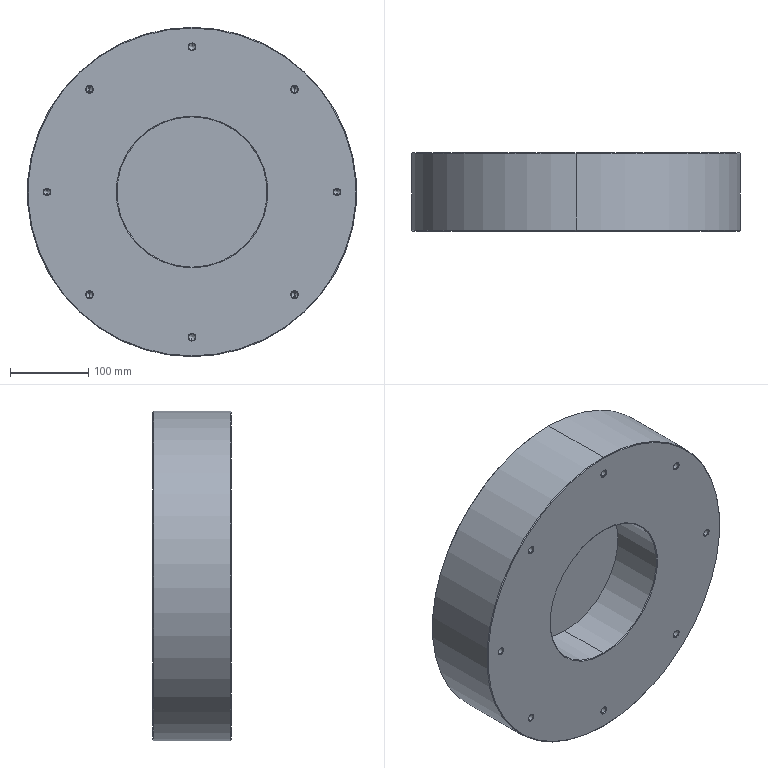Part | SolidWorks | features Chamfer 1, CirPattern 1, Extrusion 1, HoleWzd 1, ICE 1 | 1 solid | 61 faces | box 420 x 100 x 420 mm | volume 11820755 mm3 | cone 38 | cylinder 20 | plane 3 | commonest cylinder face diameters 8.5 x16 191.64 x2 420 x2
STEP:
#1=CARTESIAN_POINT('',(0.,0.,-209.));
#2=VERTEX_POINT('',#1);
#3=CARTESIAN_POINT('',(0.,0.,209.));
#4=VERTEX_POINT('',#3);
#5=CARTESIAN_POINT('',(0.,0.,0.));
#6=DIRECTION('',(0.,-1.,0.));
#7=DIRECTION('',(0.,0.,1.));
#8=AXIS2_PLACEMENT_3D('',#5,#6,#7);
#9=CIRCLE('',#8,209.);
#10=EDGE_CURVE('',#2,#4,#9,.T.);
#11=ORIENTED_EDGE('',*,*,#10,.F.);
#12=CARTESIAN_POINT('',(0.,1.,-210.));
#13=VERTEX_POINT('',#12);
#14=CARTESIAN_POINT('',(0.,1.,-210.));
#15=DIRECTION('',(0.,0.7071,-0.7071));
#16=VECTOR('',#15,1000.);
#17=LINE('',#14,#16);
#18=EDGE_CURVE('',#2,#13,#17,.T.);
#19=ORIENTED_EDGE('',*,*,#18,.T.);
#20=CARTESIAN_POINT('',(0.,1.,210.));
#21=VERTEX_POINT('',#20);
#22=CARTESIAN_POINT('',(0.,1.,0.));
#23=DIRECTION('',(0.,1.,0.));
#24=DIRECTION('',(0.,0.,1.));
#25=AXIS2_PLACEMENT_3D('',#22,#23,#24);
#26=CIRCLE('',#25,210.);
#27=EDGE_CURVE('',#21,#13,#26,.T.);
#28=ORIENTED_EDGE('',*,*,#27,.F.);
#29=CARTESIAN_POINT('',(0.,1.,210.));
#30=DIRECTION('',(0.,0.7071,0.7071));
#31=VECTOR('',#30,1000.);
#32=LINE('',#29,#31);
#33=EDGE_CURVE('',#4,#21,#32,.T.);
#34=ORIENTED_EDGE('',*,*,#33,.F.);
#35=EDGE_LOOP('',(#11,#19,#28,#34));
#36=FACE_OUTER_BOUND('',#35,.T.);
#37=CARTESIAN_POINT('',(0.,1.,0.));
#38=DIRECTION('',(0.,1.,0.));
#39=DIRECTION('',(0.,0.,1.));
#40=AXIS2_PLACEMENT_3D('',#37,#38,#39);
#41=CONICAL_SURFACE('',#40,210.,0.7854);
#42=ADVANCED_FACE('',(#36),#41,.T.);
#43=CARTESIAN_POINT('',(0.,1.,95.82));
#44=VERTEX_POINT('',#43);
#45=CARTESIAN_POINT('',(0.,1.,-95.82));
#46=VERTEX_POINT('',#45);
#47=CARTESIAN_POINT('',(0.,1.,0.));
#48=DIRECTION('',(0.,-1.,0.));
#49=DIRECTION('',(0.,0.,1.));
#50=AXIS2_PLACEMENT_3D('',#47,#48,#49);
#51=CIRCLE('',#50,95.82);
#52=EDGE_CURVE('',#44,#46,#51,.T.);
#53=ORIENTED_EDGE('',*,*,#52,.F.);
#54=CARTESIAN_POINT('',(0.,0.,96.82));
#55=VERTEX_POINT('',#54);
#56=CARTESIAN_POINT('',(0.,0.,96.82));
#57=DIRECTION('',(0.,-0.7071,0.7071));
#58=VECTOR('',#57,1000.);
#59=LINE('',#56,#58);
#60=EDGE_CURVE('',#44,#55,#59,.T.);
#61=ORIENTED_EDGE('',*,*,#60,.T.);
#62=CARTESIAN_POINT('',(0.,0.,-96.82));
#63=VERTEX_POINT('',#62);
#64=CARTESIAN_POINT('',(0.,0.,0.));
#65=DIRECTION('',(0.,1.,0.));
#66=DIRECTION('',(0.,0.,1.));
#67=AXIS2_PLACEMENT_3D('',#64,#65,#66);
#68=CIRCLE('',#67,96.82);
#69=EDGE_CURVE('',#63,#55,#68,.T.);
#70=ORIENTED_EDGE('',*,*,#69,.F.);
#71=CARTESIAN_POINT('',(0.,0.,-96.82));
#72=DIRECTION('',(0.,-0.7071,-0.7071));
#73=VECTOR('',#72,1000.);
#74=LINE('',#71,#73);
#75=EDGE_CURVE('',#46,#63,#74,.T.);
#76=ORIENTED_EDGE('',*,*,#75,.F.);
#77=EDGE_LOOP('',(#53,#61,#70,#76));
#78=FACE_OUTER_BOUND('',#77,.T.);
#79=CARTESIAN_POINT('',(0.,0.,0.));
#80=DIRECTION('',(0.,-1.,0.));
#81=DIRECTION('',(0.,0.,-1.));
#82=AXIS2_PLACEMENT_3D('',#79,#80,#81);
#83=CONICAL_SURFACE('',#82,96.82,0.7854);
#84=ADVANCED_FACE('',(#78),#83,.F.);
#85=CARTESIAN_POINT('',(0.,100.,209.));
#86=VERTEX_POINT('',#85);
#87=CARTESIAN_POINT('',(0.,100.,-209.));
#88=VERTEX_POINT('',#87);
#89=CARTESIAN_POINT('',(0.,100.,0.));
#90=DIRECTION('',(0.,1.,0.));
#91=DIRECTION('',(0.,0.,1.));
#92=AXIS2_PLACEMENT_3D('',#89,#90,#91);
#93=CIRCLE('',#92,209.);
#94=EDGE_CURVE('',#86,#88,#93,.T.);
#95=ORIENTED_EDGE('',*,*,#94,.F.);
#96=CARTESIAN_POINT('',(0.,99.,210.));
#97=VERTEX_POINT('',#96);
#98=CARTESIAN_POINT('',(0.,100.,209.));
#99=DIRECTION('',(0.,-0.7071,0.7071));
#100=VECTOR('',#99,1000.);
#101=LINE('',#98,#100);
#102=EDGE_CURVE('',#86,#97,#101,.T.);
#103=ORIENTED_EDGE('',*,*,#102,.T.);
#104=CARTESIAN_POINT('',(0.,99.,-210.));
#105=VERTEX_POINT('',#104);
#106=CARTESIAN_POINT('',(0.,99.,0.));
#107=DIRECTION('',(0.,-1.,0.));
#108=DIRECTION('',(0.,0.,1.));
#109=AXIS2_PLACEMENT_3D('',#106,#107,#108);
#110=CIRCLE('',#109,210.);
#111=EDGE_CURVE('',#105,#97,#110,.T.);
#112=ORIENTED_EDGE('',*,*,#111,.F.);
#113=CARTESIAN_POINT('',(0.,100.,-209.));
#114=DIRECTION('',(0.,-0.7071,-0.7071));
#115=VECTOR('',#114,1000.);
#116=LINE('',#113,#115);
#117=EDGE_CURVE('',#88,#105,#116,.T.);
#118=ORIENTED_EDGE('',*,*,#117,.F.);
#119=EDGE_LOOP('',(#95,#103,#112,#118));
#120=FACE_OUTER_BOUND('',#119,.T.);
#121=CARTESIAN_POINT('',(0.,100.,0.));
#122=DIRECTION('',(0.,-1.,0.));
#123=DIRECTION('',(0.,0.,-1.));
#124=AXIS2_PLACEMENT_3D('',#121,#122,#123);
#125=CONICAL_SURFACE('',#124,209.,0.7854);
#126=ADVANCED_FACE('',(#120),#125,.T.);
#127=CARTESIAN_POINT('',(130.815,0.775,135.065));
#128=VERTEX_POINT('',#127);
#129=CARTESIAN_POINT('',(130.815,0.775,126.565));
#130=VERTEX_POINT('',#129);
#131=CARTESIAN_POINT('',(130.815,0.775,130.815));
#132=DIRECTION('',(0.,-1.,0.));
#133=DIRECTION('',(0.,0.,-1.));
#134=AXIS2_PLACEMENT_3D('',#131,#132,#133);
#135=CIRCLE('',#134,4.25);
#136=EDGE_CURVE('',#128,#130,#135,.T.);
#137=ORIENTED_EDGE('',*,*,#136,.F.);
#138=CARTESIAN_POINT('',(130.815,0.,135.84));
#139=VERTEX_POINT('',#138);
#140=CARTESIAN_POINT('',(130.815,0.,135.84));
#141=DIRECTION('',(0.,-0.7071,0.7071));
#142=VECTOR('',#141,1000.);
#143=LINE('',#140,#142);
#144=EDGE_CURVE('',#128,#139,#143,.T.);
#145=ORIENTED_EDGE('',*,*,#144,.T.);
#146=CARTESIAN_POINT('',(130.815,0.,125.79));
#147=VERTEX_POINT('',#146);
#148=CARTESIAN_POINT('',(130.815,0.,130.815));
#149=DIRECTION('',(0.,-1.,0.));
#150=DIRECTION('',(0.,0.,-1.));
#151=AXIS2_PLACEMENT_3D('',#148,#149,#150);
#152=CIRCLE('',#151,5.025);
#153=EDGE_CURVE('',#139,#147,#152,.T.);
#154=ORIENTED_EDGE('',*,*,#153,.T.);
#155=CARTESIAN_POINT('',(130.815,0.,125.79));
#156=DIRECTION('',(0.,-0.7071,-0.7071));
#157=VECTOR('',#156,1000.);
#158=LINE('',#155,#157);
#159=EDGE_CURVE('',#130,#147,#158,.T.);
#160=ORIENTED_EDGE('',*,*,#159,.F.);
#161=EDGE_LOOP('',(#137,#145,#154,#160));
#162=FACE_OUTER_BOUND('',#161,.T.);
#163=CARTESIAN_POINT('',(130.815,0.,130.815));
#164=DIRECTION('',(0.,-1.,0.));
#165=DIRECTION('',(0.,0.,-1.));
#166=AXIS2_PLACEMENT_3D('',#163,#164,#165);
#167=CONICAL_SURFACE('',#166,5.025,0.7854);
#168=ADVANCED_FACE('',(#162),#167,.F.);
#169=CARTESIAN_POINT('',(130.815,27.5,135.065));
#170=VERTEX_POINT('',#169);
#171=CARTESIAN_POINT('',(130.815,27.5,126.565));
#172=VERTEX_POINT('',#171);
#173=CARTESIAN_POINT('',(130.815,27.5,130.815));
#174=DIRECTION('',(0.,-1.,0.));
#175=DIRECTION('',(0.,0.,-1.));
#176=AXIS2_PLACEMENT_3D('',#173,#174,#175);
#177=CIRCLE('',#176,4.25);
#178=EDGE_CURVE('',#170,#172,#177,.T.);
#179=ORIENTED_EDGE('',*,*,#178,.F.);
#180=CARTESIAN_POINT('',(130.815,0.,135.065));
#181=DIRECTION('',(0.,-1.,0.));
#182=VECTOR('',#181,1000.);
#183=LINE('',#180,#182);
#184=EDGE_CURVE('',#170,#128,#183,.T.);
#185=ORIENTED_EDGE('',*,*,#184,.T.);
#186=ORIENTED_EDGE('',*,*,#136,.T.);
#187=CARTESIAN_POINT('',(130.815,0.,126.565));
#188=DIRECTION('',(0.,-1.,0.));
#189=VECTOR('',#188,1000.);
#190=LINE('',#187,#189);
#191=EDGE_CURVE('',#172,#130,#190,.T.);
#192=ORIENTED_EDGE('',*,*,#191,.F.);
#193=EDGE_LOOP('',(#179,#185,#186,#192));
#194=FACE_OUTER_BOUND('',#193,.T.);
#195=CARTESIAN_POINT('',(130.815,0.,130.815));
#196=DIRECTION('',(0.,-1.,0.));
#197=DIRECTION('',(0.,0.,-1.));
#198=AXIS2_PLACEMENT_3D('',#195,#196,#197);
#199=CYLINDRICAL_SURFACE('',#198,4.25);
#200=ADVANCED_FACE('',(#194),#199,.F.);
#201=CARTESIAN_POINT('',(130.815,30.054,130.815));
#202=VERTEX_POINT('',#201);
#203=CARTESIAN_POINT('',(130.815,27.5,126.565));
#204=DIRECTION('',(0.,-0.515,-0.8572));
#205=VECTOR('',#204,1000.);
#206=LINE('',#203,#205);
#207=EDGE_CURVE('',#202,#172,#206,.T.);
#208=ORIENTED_EDGE('',*,*,#207,.F.);
#209=CARTESIAN_POINT('',(130.815,27.5,135.065));
#210=DIRECTION('',(0.,-0.515,0.8572));
#211=VECTOR('',#210,1000.);
#212=LINE('',#209,#211);
#213=EDGE_CURVE('',#202,#170,#212,.T.);
#214=ORIENTED_EDGE('',*,*,#213,.T.);
#215=ORIENTED_EDGE('',*,*,#178,.T.);
#216=EDGE_LOOP('',(#208,#214,#215));
#217=FACE_OUTER_BOUND('',#216,.T.);
#218=CARTESIAN_POINT('',(130.815,27.5,130.815));
#219=DIRECTION('',(0.,-1.,0.));
#220=DIRECTION('',(0.,0.,-1.));
#221=AXIS2_PLACEMENT_3D('',#218,#219,#220);
#222=CONICAL_SURFACE('',#221,4.25,1.03);
#223=ADVANCED_FACE('',(#217),#222,.F.);
#224=CARTESIAN_POINT('',(0.,0.775,189.25));
#225=VERTEX_POINT('',#224);
#226=CARTESIAN_POINT('',(0.,0.775,180.75));
#227=VERTEX_POINT('',#226);
#228=CARTESIAN_POINT('',(0.,0.775,185.));
#229=DIRECTION('',(0.,-1.,0.));
#230=DIRECTION('',(0.,0.,-1.));
#231=AXIS2_PLACEMENT_3D('',#228,#229,#230);
#232=CIRCLE('',#231,4.25);
#233=EDGE_CURVE('',#225,#227,#232,.T.);
#234=ORIENTED_EDGE('',*,*,#233,.F.);
#235=CARTESIAN_POINT('',(0.,0.,190.025));
#236=VERTEX_POINT('',#235);
#237=CARTESIAN_POINT('',(0.,0.,190.025));
#238=DIRECTION('',(0.,-0.7071,0.7071));
#239=VECTOR('',#238,1000.);
#240=LINE('',#237,#239);
#241=EDGE_CURVE('',#225,#236,#240,.T.);
#242=ORIENTED_EDGE('',*,*,#241,.T.);
#243=CARTESIAN_POINT('',(0.,0.,179.975));
#244=VERTEX_POINT('',#243);
#245=CARTESIAN_POINT('',(0.,0.,185.));
#246=DIRECTION('',(0.,-1.,0.));
#247=DIRECTION('',(0.,0.,-1.));
#248=AXIS2_PLACEMENT_3D('',#245,#246,#247);
#249=CIRCLE('',#248,5.025);
#250=EDGE_CURVE('',#236,#244,#249,.T.);
#251=ORIENTED_EDGE('',*,*,#250,.T.);
#252=CARTESIAN_POINT('',(0.,0.,179.975));
#253=DIRECTION('',(0.,-0.7071,-0.7071));
#254=VECTOR('',#253,1000.);
#255=LINE('',#252,#254);
#256=EDGE_CURVE('',#227,#244,#255,.T.);
#257=ORIENTED_EDGE('',*,*,#256,.F.);
#258=EDGE_LOOP('',(#234,#242,#251,#257));
#259=FACE_OUTER_BOUND('',#258,.T.);
#260=CARTESIAN_POINT('',(0.,0.,185.));
#261=DIRECTION('',(0.,-1.,0.));
#262=DIRECTION('',(0.,0.,-1.));
#263=AXIS2_PLACEMENT_3D('',#260,#261,#262);
#264=CONICAL_SURFACE('',#263,5.025,0.7854);
#265=ADVANCED_FACE('',(#259),#264,.F.);
#266=CARTESIAN_POINT('',(0.,27.5,189.25));
#267=VERTEX_POINT('',#266);
#268=CARTESIAN_POINT('',(0.,27.5,180.75));
#269=VERTEX_POINT('',#268);
#270=CARTESIAN_POINT('',(0.,27.5,185.));
#271=DIRECTION('',(0.,-1.,0.));
#272=DIRECTION('',(0.,0.,-1.));
#273=AXIS2_PLACEMENT_3D('',#270,#271,#272);
#274=CIRCLE('',#273,4.25);
#275=EDGE_CURVE('',#267,#269,#274,.T.);
#276=ORIENTED_EDGE('',*,*,#275,.F.);
#277=CARTESIAN_POINT('',(0.,0.,189.25));
#278=DIRECTION('',(0.,-1.,0.));
#279=VECTOR('',#278,1000.);
#280=LINE('',#277,#279);
#281=EDGE_CURVE('',#267,#225,#280,.T.);
#282=ORIENTED_EDGE('',*,*,#281,.T.);
#283=ORIENTED_EDGE('',*,*,#233,.T.);
#284=CARTESIAN_POINT('',(0.,0.,180.75));
#285=DIRECTION('',(0.,-1.,0.));
#286=VECTOR('',#285,1000.);
#287=LINE('',#284,#286);
#288=EDGE_CURVE('',#269,#227,#287,.T.);
#289=ORIENTED_EDGE('',*,*,#288,.F.);
#290=EDGE_LOOP('',(#276,#282,#283,#289));
#291=FACE_OUTER_BOUND('',#290,.T.);
#292=CARTESIAN_POINT('',(0.,0.,185.));
#293=DIRECTION('',(0.,-1.,0.));
#294=DIRECTION('',(0.,0.,-1.));
#295=AXIS2_PLACEMENT_3D('',#292,#293,#294);
#296=CYLINDRICAL_SURFACE('',#295,4.25);
#297=ADVANCED_FACE('',(#291),#296,.F.);
#298=CARTESIAN_POINT('',(0.,30.054,185.));
#299=VERTEX_POINT('',#298);
#300=CARTESIAN_POINT('',(0.,27.5,180.75));
#301=DIRECTION('',(0.,-0.515,-0.8572));
#302=VECTOR('',#301,1000.);
#303=LINE('',#300,#302);
#304=EDGE_CURVE('',#299,#269,#303,.T.);
#305=ORIENTED_EDGE('',*,*,#304,.F.);
#306=CARTESIAN_POINT('',(0.,27.5,189.25));
#307=DIRECTION('',(0.,-0.515,0.8572));
#308=VECTOR('',#307,1000.);
#309=LINE('',#306,#308);
#310=EDGE_CURVE('',#299,#267,#309,.T.);
#311=ORIENTED_EDGE('',*,*,#310,.T.);
#312=ORIENTED_EDGE('',*,*,#275,.T.);
#313=EDGE_LOOP('',(#305,#311,#312));
#314=FACE_OUTER_BOUND('',#313,.T.);
#315=CARTESIAN_POINT('',(0.,27.5,185.));
#316=DIRECTION('',(0.,-1.,0.));
#317=DIRECTION('',(0.,0.,-1.));
#318=AXIS2_PLACEMENT_3D('',#315,#316,#317);
#319=CONICAL_SURFACE('',#318,4.25,1.03);
#320=ADVANCED_FACE('',(#314),#319,.F.);
#321=CARTESIAN_POINT('',(-130.815,0.775,135.065));
#322=VERTEX_POINT('',#321);
#323=CARTESIAN_POINT('',(-130.815,0.775,126.565));
#324=VERTEX_POINT('',#323);
#325=CARTESIAN_POINT('',(-130.815,0.775,130.815));
#326=DIRECTION('',(0.,-1.,0.));
#327=DIRECTION('',(0.,0.,-1.));
#328=AXIS2_PLACEMENT_3D('',#325,#326,#327);
#329=CIRCLE('',#328,4.25);
#330=EDGE_CURVE('',#322,#324,#329,.T.);
#331=ORIENTED_EDGE('',*,*,#330,.F.);
#332=CARTESIAN_POINT('',(-130.815,0.,135.84));
#333=VERTEX_POINT('',#332);
#334=CARTESIAN_POINT('',(-130.815,0.,135.84));
#335=DIRECTION('',(0.,-0.7071,0.7071));
#336=VECTOR('',#335,1000.);
#337=LINE('',#334,#336);
#338=EDGE_CURVE('',#322,#333,#337,.T.);
#339=ORIENTED_EDGE('',*,*,#338,.T.);
#340=CARTESIAN_POINT('',(-130.815,0.,125.79));
#341=VERTEX_POINT('',#340);
#342=CARTESIAN_POINT('',(-130.815,0.,130.815));
#343=DIRECTION('',(0.,-1.,0.));
#344=DIRECTION('',(0.,0.,-1.));
#345=AXIS2_PLACEMENT_3D('',#342,#343,#344);
#346=CIRCLE('',#345,5.025);
#347=EDGE_CURVE('',#333,#341,#346,.T.);
#348=ORIENTED_EDGE('',*,*,#347,.T.);
#349=CARTESIAN_POINT('',(-130.815,0.,125.79));
#350=DIRECTION('',(0.,-0.7071,-0.7071));
#351=VECTOR('',#350,1000.);
#352=LINE('',#349,#351);
#353=EDGE_CURVE('',#324,#341,#352,.T.);
#354=ORIENTED_EDGE('',*,*,#353,.F.);
#355=EDGE_LOOP('',(#331,#339,#348,#354));
#356=FACE_OUTER_BOUND('',#355,.T.);
#357=CARTESIAN_POINT('',(-130.815,0.,130.815));
#358=DIRECTION('',(0.,-1.,0.));
#359=DIRECTION('',(0.,0.,-1.));
#360=AXIS2_PLACEMENT_3D('',#357,#358,#359);
#361=CONICAL_SURFACE('',#360,5.025,0.7854);
#362=ADVANCED_FACE('',(#356),#361,.F.);
#363=CARTESIAN_POINT('',(-130.815,27.5,135.065));
#364=VERTEX_POINT('',#363);
#365=CARTESIAN_POINT('',(-130.815,27.5,126.565));
#366=VERTEX_POINT('',#365);
#367=CARTESIAN_POINT('',(-130.815,27.5,130.815));
#368=DIRECTION('',(0.,-1.,0.));
#369=DIRECTION('',(0.,0.,-1.));
#370=AXIS2_PLACEMENT_3D('',#367,#368,#369);
#371=CIRCLE('',#370,4.25);
#372=EDGE_CURVE('',#364,#366,#371,.T.);
#373=ORIENTED_EDGE('',*,*,#372,.F.);
#374=CARTESIAN_POINT('',(-130.815,0.,135.065));
#375=DIRECTION('',(0.,-1.,0.));
#376=VECTOR('',#375,1000.);
#377=LINE('',#374,#376);
#378=EDGE_CURVE('',#364,#322,#377,.T.);
#379=ORIENTED_EDGE('',*,*,#378,.T.);
#380=ORIENTED_EDGE('',*,*,#330,.T.);
#381=CARTESIAN_POINT('',(-130.815,0.,126.565));
#382=DIRECTION('',(0.,-1.,0.));
#383=VECTOR('',#382,1000.);
#384=LINE('',#381,#383);
#385=EDGE_CURVE('',#366,#324,#384,.T.);
#386=ORIENTED_EDGE('',*,*,#385,.F.);
#387=EDGE_LOOP('',(#373,#379,#380,#386));
#388=FACE_OUTER_BOUND('',#387,.T.);
#389=CARTESIAN_POINT('',(-130.815,0.,130.815));
#390=DIRECTION('',(0.,-1.,0.));
#391=DIRECTION('',(0.,0.,-1.));
#392=AXIS2_PLACEMENT_3D('',#389,#390,#391);
#393=CYLINDRICAL_SURFACE('',#392,4.25);
#394=ADVANCED_FACE('',(#388),#393,.F.);
#395=CARTESIAN_POINT('',(-130.815,30.054,130.815));
#396=VERTEX_POINT('',#395);
#397=CARTESIAN_POINT('',(-130.815,27.5,126.565));
#398=DIRECTION('',(0.,-0.515,-0.8572));
#399=VECTOR('',#398,1000.);
#400=LINE('',#397,#399);
#401=EDGE_CURVE('',#396,#366,#400,.T.);
#402=ORIENTED_EDGE('',*,*,#401,.F.);
#403=CARTESIAN_POINT('',(-130.815,27.5,135.065));
#404=DIRECTION('',(0.,-0.515,0.8572));
#405=VECTOR('',#404,1000.);
#406=LINE('',#403,#405);
#407=EDGE_CURVE('',#396,#364,#406,.T.);
#408=ORIENTED_EDGE('',*,*,#407,.T.);
#409=ORIENTED_EDGE('',*,*,#372,.T.);
#410=EDGE_LOOP('',(#402,#408,#409));
#411=FACE_OUTER_BOUND('',#410,.T.);
#412=CARTESIAN_POINT('',(-130.815,27.5,130.815));
#413=DIRECTION('',(0.,-1.,0.));
#414=DIRECTION('',(0.,0.,-1.));
#415=AXIS2_PLACEMENT_3D('',#412,#413,#414);
#416=CONICAL_SURFACE('',#415,4.25,1.03);
#417=ADVANCED_FACE('',(#411),#416,.F.);
#418=CARTESIAN_POINT('',(-185.,0.775,4.25));
#419=VERTEX_POINT('',#418);
#420=CARTESIAN_POINT('',(-185.,0.775,-4.25));
#421=VERTEX_POINT('',#420);
#422=CARTESIAN_POINT('',(-185.,0.775,0.));
#423=DIRECTION('',(0.,-1.,0.));
#424=DIRECTION('',(0.,0.,-1.));
#425=AXIS2_PLACEMENT_3D('',#422,#423,#424);
#426=CIRCLE('',#425,4.25);
#427=EDGE_CURVE('',#419,#421,#426,.T.);
#428=ORIENTED_EDGE('',*,*,#427,.F.);
#429=CARTESIAN_POINT('',(-185.,0.,5.025));
#430=VERTEX_POINT('',#429);
#431=CARTESIAN_POINT('',(-185.,0.,5.025));
#432=DIRECTION('',(0.,-0.7071,0.7071));
#433=VECTOR('',#432,1000.);
#434=LINE('',#431,#433);
#435=EDGE_CURVE('',#419,#430,#434,.T.);
#436=ORIENTED_EDGE('',*,*,#435,.T.);
#437=CARTESIAN_POINT('',(-185.,0.,-5.025));
#438=VERTEX_POINT('',#437);
#439=CARTESIAN_POINT('',(-185.,0.,0.));
#440=DIRECTION('',(0.,-1.,0.));
#441=DIRECTION('',(0.,0.,-1.));
#442=AXIS2_PLACEMENT_3D('',#439,#440,#441);
#443=CIRCLE('',#442,5.025);
#444=EDGE_CURVE('',#430,#438,#443,.T.);
#445=ORIENTED_EDGE('',*,*,#444,.T.);
#446=CARTESIAN_POINT('',(-185.,0.,-5.025));
#447=DIRECTION('',(0.,-0.7071,-0.7071));
#448=VECTOR('',#447,1000.);
#449=LINE('',#446,#448);
#450=EDGE_CURVE('',#421,#438,#449,.T.);
#451=ORIENTED_EDGE('',*,*,#450,.F.);
#452=EDGE_LOOP('',(#428,#436,#445,#451));
#453=FACE_OUTER_BOUND('',#452,.T.);
#454=CARTESIAN_POINT('',(-185.,0.,0.));
#455=DIRECTION('',(0.,-1.,0.));
#456=DIRECTION('',(0.,0.,-1.));
#457=AXIS2_PLACEMENT_3D('',#454,#455,#456);
#458=CONICAL_SURFACE('',#457,5.025,0.7854);
#459=ADVANCED_FACE('',(#453),#458,.F.);
#460=CARTESIAN_POINT('',(-185.,27.5,4.25));
#461=VERTEX_POINT('',#460);
#462=CARTESIAN_POINT('',(-185.,27.5,-4.25));
#463=VERTEX_POINT('',#462);
#464=CARTESIAN_POINT('',(-185.,27.5,0.));
#465=DIRECTION('',(0.,-1.,0.));
#466=DIRECTION('',(0.,0.,-1.));
#467=AXIS2_PLACEMENT_3D('',#464,#465,#466);
#468=CIRCLE('',#467,4.25);
#469=EDGE_CURVE('',#461,#463,#468,.T.);
#470=ORIENTED_EDGE('',*,*,#469,.F.);
#471=CARTESIAN_POINT('',(-185.,0.,4.25));
#472=DIRECTION('',(0.,-1.,0.));
#473=VECTOR('',#472,1000.);
#474=LINE('',#471,#473);
#475=EDGE_CURVE('',#461,#419,#474,.T.);
#476=ORIENTED_EDGE('',*,*,#475,.T.);
#477=ORIENTED_EDGE('',*,*,#427,.T.);
#478=CARTESIAN_POINT('',(-185.,0.,-4.25));
#479=DIRECTION('',(0.,-1.,0.));
#480=VECTOR('',#479,1000.);
#481=LINE('',#478,#480);
#482=EDGE_CURVE('',#463,#421,#481,.T.);
#483=ORIENTED_EDGE('',*,*,#482,.F.);
#484=EDGE_LOOP('',(#470,#476,#477,#483));
#485=FACE_OUTER_BOUND('',#484,.T.);
#486=CARTESIAN_POINT('',(-185.,0.,0.));
#487=DIRECTION('',(0.,-1.,0.));
#488=DIRECTION('',(0.,0.,-1.));
#489=AXIS2_PLACEMENT_3D('',#486,#487,#488);
#490=CYLINDRICAL_SURFACE('',#489,4.25);
#491=ADVANCED_FACE('',(#485),#490,.F.);
#492=CARTESIAN_POINT('',(-185.,30.054,0.));
#493=VERTEX_POINT('',#492);
#494=CARTESIAN_POINT('',(-185.,27.5,-4.25));
#495=DIRECTION('',(0.,-0.515,-0.8572));
#496=VECTOR('',#495,1000.);
#497=LINE('',#494,#496);
#498=EDGE_CURVE('',#493,#463,#497,.T.);
#499=ORIENTED_EDGE('',*,*,#498,.F.);
#500=CARTESIAN_POINT('',(-185.,27.5,4.25));
#501=DIRECTION('',(0.,-0.515,0.8572));
#502=VECTOR('',#501,1000.);
#503=LINE('',#500,#502);
#504=EDGE_CURVE('',#493,#461,#503,.T.);
#505=ORIENTED_EDGE('',*,*,#504,.T.);
#506=ORIENTED_EDGE('',*,*,#469,.T.);
#507=EDGE_LOOP('',(#499,#505,#506));
#508=FACE_OUTER_BOUND('',#507,.T.);
#509=CARTESIAN_POINT('',(-185.,27.5,0.));
#510=DIRECTION('',(0.,-1.,0.));
#511=DIRECTION('',(0.,0.,-1.));
#512=AXIS2_PLACEMENT_3D('',#509,#510,#511);
#513=CONICAL_SURFACE('',#512,4.25,1.03);
#514=ADVANCED_FACE('',(#508),#513,.F.);
#515=CARTESIAN_POINT('',(-130.815,0.775,-126.565));
#516=VERTEX_POINT('',#515);
#517=CARTESIAN_POINT('',(-130.815,0.775,-135.065));
#518=VERTEX_POINT('',#517);
#519=CARTESIAN_POINT('',(-130.815,0.775,-130.815));
#520=DIRECTION('',(0.,-1.,0.));
#521=DIRECTION('',(0.,0.,-1.));
#522=AXIS2_PLACEMENT_3D('',#519,#520,#521);
#523=CIRCLE('',#522,4.25);
#524=EDGE_CURVE('',#516,#518,#523,.T.);
#525=ORIENTED_EDGE('',*,*,#524,.F.);
#526=CARTESIAN_POINT('',(-130.815,0.,-125.79));
#527=VERTEX_POINT('',#526);
#528=CARTESIAN_POINT('',(-130.815,0.,-125.79));
#529=DIRECTION('',(0.,-0.7071,0.7071));
#530=VECTOR('',#529,1000.);
#531=LINE('',#528,#530);
#532=EDGE_CURVE('',#516,#527,#531,.T.);
#533=ORIENTED_EDGE('',*,*,#532,.T.);
#534=CARTESIAN_POINT('',(-130.815,0.,-135.84));
#535=VERTEX_POINT('',#534);
#536=CARTESIAN_POINT('',(-130.815,0.,-130.815));
#537=DIRECTION('',(0.,-1.,0.));
#538=DIRECTION('',(0.,0.,-1.));
#539=AXIS2_PLACEMENT_3D('',#536,#537,#538);
#540=CIRCLE('',#539,5.025);
#541=EDGE_CURVE('',#527,#535,#540,.T.);
#542=ORIENTED_EDGE('',*,*,#541,.T.);
#543=CARTESIAN_POINT('',(-130.815,0.,-135.84));
#544=DIRECTION('',(0.,-0.7071,-0.7071));
#545=VECTOR('',#544,1000.);
#546=LINE('',#543,#545);
#547=EDGE_CURVE('',#518,#535,#546,.T.);
#548=ORIENTED_EDGE('',*,*,#547,.F.);
#549=EDGE_LOOP('',(#525,#533,#542,#548));
#550=FACE_OUTER_BOUND('',#549,.T.);
#551=CARTESIAN_POINT('',(-130.815,0.,-130.815));
#552=DIRECTION('',(0.,-1.,0.));
#553=DIRECTION('',(0.,0.,-1.));
#554=AXIS2_PLACEMENT_3D('',#551,#552,#553);
#555=CONICAL_SURFACE('',#554,5.025,0.7854);
#556=ADVANCED_FACE('',(#550),#555,.F.);
#557=CARTESIAN_POINT('',(-130.815,27.5,-126.565));
#558=VERTEX_POINT('',#557);
#559=CARTESIAN_POINT('',(-130.815,27.5,-135.065));
#560=VERTEX_POINT('',#559);
#561=CARTESIAN_POINT('',(-130.815,27.5,-130.815));
#562=DIRECTION('',(0.,-1.,0.));
#563=DIRECTION('',(0.,0.,-1.));
#564=AXIS2_PLACEMENT_3D('',#561,#562,#563);
#565=CIRCLE('',#564,4.25);
#566=EDGE_CURVE('',#558,#560,#565,.T.);
#567=ORIENTED_EDGE('',*,*,#566,.F.);
#568=CARTESIAN_POINT('',(-130.815,0.,-126.565));
#569=DIRECTION('',(0.,-1.,0.));
#570=VECTOR('',#569,1000.);
#571=LINE('',#568,#570);
#572=EDGE_CURVE('',#558,#516,#571,.T.);
#573=ORIENTED_EDGE('',*,*,#572,.T.);
#574=ORIENTED_EDGE('',*,*,#524,.T.);
#575=CARTESIAN_POINT('',(-130.815,0.,-135.065));
#576=DIRECTION('',(0.,-1.,0.));
#577=VECTOR('',#576,1000.);
#578=LINE('',#575,#577);
#579=EDGE_CURVE('',#560,#518,#578,.T.);
#580=ORIENTED_EDGE('',*,*,#579,.F.);
#581=EDGE_LOOP('',(#567,#573,#574,#580));
#582=FACE_OUTER_BOUND('',#581,.T.);
#583=CARTESIAN_POINT('',(-130.815,0.,-130.815));
#584=DIRECTION('',(0.,-1.,0.));
#585=DIRECTION('',(0.,0.,-1.));
#586=AXIS2_PLACEMENT_3D('',#583,#584,#585);
#587=CYLINDRICAL_SURFACE('',#586,4.25);
#588=ADVANCED_FACE('',(#582),#587,.F.);
#589=CARTESIAN_POINT('',(-130.815,30.054,-130.815));
#590=VERTEX_POINT('',#589);
#591=CARTESIAN_POINT('',(-130.815,27.5,-135.065));
#592=DIRECTION('',(0.,-0.515,-0.8572));
#593=VECTOR('',#592,1000.);
#594=LINE('',#591,#593);
#595=EDGE_CURVE('',#590,#560,#594,.T.);
#596=ORIENTED_EDGE('',*,*,#595,.F.);
#597=CARTESIAN_POINT('',(-130.815,27.5,-126.565));
#598=DIRECTION('',(0.,-0.515,0.8572));
#599=VECTOR('',#598,1000.);
#600=LINE('',#597,#599);
#601=EDGE_CURVE('',#590,#558,#600,.T.);
#602=ORIENTED_EDGE('',*,*,#601,.T.);
#603=ORIENTED_EDGE('',*,*,#566,.T.);
#604=EDGE_LOOP('',(#596,#602,#603));
#605=FACE_OUTER_BOUND('',#604,.T.);
#606=CARTESIAN_POINT('',(-130.815,27.5,-130.815));
#607=DIRECTION('',(0.,-1.,0.));
#608=DIRECTION('',(0.,0.,-1.));
#609=AXIS2_PLACEMENT_3D('',#606,#607,#608);
#610=CONICAL_SURFACE('',#609,4.25,1.03);
#611=ADVANCED_FACE('',(#605),#610,.F.);
#612=CARTESIAN_POINT('',(0.,0.775,-180.75));
#613=VERTEX_POINT('',#612);
#614=CARTESIAN_POINT('',(0.,0.775,-189.25));
#615=VERTEX_POINT('',#614);
#616=CARTESIAN_POINT('',(0.,0.775,-185.));
#617=DIRECTION('',(0.,-1.,0.));
#618=DIRECTION('',(0.,0.,-1.));
#619=AXIS2_PLACEMENT_3D('',#616,#617,#618);
#620=CIRCLE('',#619,4.25);
#621=EDGE_CURVE('',#613,#615,#620,.T.);
#622=ORIENTED_EDGE('',*,*,#621,.F.);
#623=CARTESIAN_POINT('',(0.,0.,-179.975));
#624=VERTEX_POINT('',#623);
#625=CARTESIAN_POINT('',(0.,0.,-179.975));
#626=DIRECTION('',(0.,-0.7071,0.7071));
#627=VECTOR('',#626,1000.);
#628=LINE('',#625,#627);
#629=EDGE_CURVE('',#613,#624,#628,.T.);
#630=ORIENTED_EDGE('',*,*,#629,.T.);
#631=CARTESIAN_POINT('',(0.,0.,-190.025));
#632=VERTEX_POINT('',#631);
#633=CARTESIAN_POINT('',(0.,0.,-185.));
#634=DIRECTION('',(0.,-1.,0.));
#635=DIRECTION('',(0.,0.,-1.));
#636=AXIS2_PLACEMENT_3D('',#633,#634,#635);
#637=CIRCLE('',#636,5.025);
#638=EDGE_CURVE('',#624,#632,#637,.T.);
#639=ORIENTED_EDGE('',*,*,#638,.T.);
#640=CARTESIAN_POINT('',(0.,0.,-190.025));
#641=DIRECTION('',(0.,-0.7071,-0.7071));
#642=VECTOR('',#641,1000.);
#643=LINE('',#640,#642);
#644=EDGE_CURVE('',#615,#632,#643,.T.);
#645=ORIENTED_EDGE('',*,*,#644,.F.);
#646=EDGE_LOOP('',(#622,#630,#639,#645));
#647=FACE_OUTER_BOUND('',#646,.T.);
#648=CARTESIAN_POINT('',(0.,0.,-185.));
#649=DIRECTION('',(0.,-1.,0.));
#650=DIRECTION('',(0.,0.,-1.));
#651=AXIS2_PLACEMENT_3D('',#648,#649,#650);
#652=CONICAL_SURFACE('',#651,5.025,0.7854);
#653=ADVANCED_FACE('',(#647),#652,.F.);
#654=CARTESIAN_POINT('',(0.,27.5,-180.75));
#655=VERTEX_POINT('',#654);
#656=CARTESIAN_POINT('',(0.,27.5,-189.25));
#657=VERTEX_POINT('',#656);
#658=CARTESIAN_POINT('',(0.,27.5,-185.));
#659=DIRECTION('',(0.,-1.,0.));
#660=DIRECTION('',(0.,0.,-1.));
#661=AXIS2_PLACEMENT_3D('',#658,#659,#660);
#662=CIRCLE('',#661,4.25);
#663=EDGE_CURVE('',#655,#657,#662,.T.);
#664=ORIENTED_EDGE('',*,*,#663,.F.);
#665=CARTESIAN_POINT('',(0.,0.,-180.75));
#666=DIRECTION('',(0.,-1.,0.));
#667=VECTOR('',#666,1000.);
#668=LINE('',#665,#667);
#669=EDGE_CURVE('',#655,#613,#668,.T.);
#670=ORIENTED_EDGE('',*,*,#669,.T.);
#671=ORIENTED_EDGE('',*,*,#621,.T.);
#672=CARTESIAN_POINT('',(0.,0.,-189.25));
#673=DIRECTION('',(0.,-1.,0.));
#674=VECTOR('',#673,1000.);
#675=LINE('',#672,#674);
#676=EDGE_CURVE('',#657,#615,#675,.T.);
#677=ORIENTED_EDGE('',*,*,#676,.F.);
#678=EDGE_LOOP('',(#664,#670,#671,#677));
#679=FACE_OUTER_BOUND('',#678,.T.);
#680=CARTESIAN_POINT('',(0.,0.,-185.));
#681=DIRECTION('',(0.,-1.,0.));
#682=DIRECTION('',(0.,0.,-1.));
#683=AXIS2_PLACEMENT_3D('',#680,#681,#682);
#684=CYLINDRICAL_SURFACE('',#683,4.25);
#685=ADVANCED_FACE('',(#679),#684,.F.);
#686=CARTESIAN_POINT('',(0.,30.054,-185.));
#687=VERTEX_POINT('',#686);
#688=CARTESIAN_POINT('',(0.,27.5,-189.25));
#689=DIRECTION('',(0.,-0.515,-0.8572));
#690=VECTOR('',#689,1000.);
#691=LINE('',#688,#690);
#692=EDGE_CURVE('',#687,#657,#691,.T.);
#693=ORIENTED_EDGE('',*,*,#692,.F.);
#694=CARTESIAN_POINT('',(0.,27.5,-180.75));
#695=DIRECTION('',(0.,-0.515,0.8572));
#696=VECTOR('',#695,1000.);
#697=LINE('',#694,#696);
#698=EDGE_CURVE('',#687,#655,#697,.T.);
#699=ORIENTED_EDGE('',*,*,#698,.T.);
#700=ORIENTED_EDGE('',*,*,#663,.T.);
#701=EDGE_LOOP('',(#693,#699,#700));
#702=FACE_OUTER_BOUND('',#701,.T.);
#703=CARTESIAN_POINT('',(0.,27.5,-185.));
#704=DIRECTION('',(0.,-1.,0.));
#705=DIRECTION('',(0.,0.,-1.));
#706=AXIS2_PLACEMENT_3D('',#703,#704,#705);
#707=CONICAL_SURFACE('',#706,4.25,1.03);
#708=ADVANCED_FACE('',(#702),#707,.F.);
#709=CARTESIAN_POINT('',(130.815,0.775,-126.565));
#710=VERTEX_POINT('',#709);
#711=CARTESIAN_POINT('',(130.815,0.775,-135.065));
#712=VERTEX_POINT('',#711);
#713=CARTESIAN_POINT('',(130.815,0.775,-130.815));
#714=DIRECTION('',(0.,-1.,0.));
#715=DIRECTION('',(0.,0.,-1.));
#716=AXIS2_PLACEMENT_3D('',#713,#714,#715);
#717=CIRCLE('',#716,4.25);
#718=EDGE_CURVE('',#710,#712,#717,.T.);
#719=ORIENTED_EDGE('',*,*,#718,.F.);
#720=CARTESIAN_POINT('',(130.815,0.,-125.79));
#721=VERTEX_POINT('',#720);
#722=CARTESIAN_POINT('',(130.815,0.,-125.79));
#723=DIRECTION('',(0.,-0.7071,0.7071));
#724=VECTOR('',#723,1000.);
#725=LINE('',#722,#724);
#726=EDGE_CURVE('',#710,#721,#725,.T.);
#727=ORIENTED_EDGE('',*,*,#726,.T.);
#728=CARTESIAN_POINT('',(130.815,0.,-135.84));
#729=VERTEX_POINT('',#728);
#730=CARTESIAN_POINT('',(130.815,0.,-130.815));
#731=DIRECTION('',(0.,-1.,0.));
#732=DIRECTION('',(0.,0.,-1.));
#733=AXIS2_PLACEMENT_3D('',#730,#731,#732);
#734=CIRCLE('',#733,5.025);
#735=EDGE_CURVE('',#721,#729,#734,.T.);
#736=ORIENTED_EDGE('',*,*,#735,.T.);
#737=CARTESIAN_POINT('',(130.815,0.,-135.84));
#738=DIRECTION('',(0.,-0.7071,-0.7071));
#739=VECTOR('',#738,1000.);
#740=LINE('',#737,#739);
#741=EDGE_CURVE('',#712,#729,#740,.T.);
#742=ORIENTED_EDGE('',*,*,#741,.F.);
#743=EDGE_LOOP('',(#719,#727,#736,#742));
#744=FACE_OUTER_BOUND('',#743,.T.);
#745=CARTESIAN_POINT('',(130.815,0.,-130.815));
#746=DIRECTION('',(0.,-1.,0.));
#747=DIRECTION('',(0.,0.,-1.));
#748=AXIS2_PLACEMENT_3D('',#745,#746,#747);
#749=CONICAL_SURFACE('',#748,5.025,0.7854);
#750=ADVANCED_FACE('',(#744),#749,.F.);
#751=CARTESIAN_POINT('',(130.815,27.5,-126.565));
#752=VERTEX_POINT('',#751);
#753=CARTESIAN_POINT('',(130.815,27.5,-135.065));
#754=VERTEX_POINT('',#753);
#755=CARTESIAN_POINT('',(130.815,27.5,-130.815));
#756=DIRECTION('',(0.,-1.,0.));
#757=DIRECTION('',(0.,0.,-1.));
#758=AXIS2_PLACEMENT_3D('',#755,#756,#757);
#759=CIRCLE('',#758,4.25);
#760=EDGE_CURVE('',#752,#754,#759,.T.);
#761=ORIENTED_EDGE('',*,*,#760,.F.);
#762=CARTESIAN_POINT('',(130.815,0.,-126.565));
#763=DIRECTION('',(0.,-1.,0.));
#764=VECTOR('',#763,1000.);
#765=LINE('',#762,#764);
#766=EDGE_CURVE('',#752,#710,#765,.T.);
#767=ORIENTED_EDGE('',*,*,#766,.T.);
#768=ORIENTED_EDGE('',*,*,#718,.T.);
#769=CARTESIAN_POINT('',(130.815,0.,-135.065));
#770=DIRECTION('',(0.,-1.,0.));
#771=VECTOR('',#770,1000.);
#772=LINE('',#769,#771);
#773=EDGE_CURVE('',#754,#712,#772,.T.);
#774=ORIENTED_EDGE('',*,*,#773,.F.);
#775=EDGE_LOOP('',(#761,#767,#768,#774));
#776=FACE_OUTER_BOUND('',#775,.T.);
#777=CARTESIAN_POINT('',(130.815,0.,-130.815));
#778=DIRECTION('',(0.,-1.,0.));
#779=DIRECTION('',(0.,0.,-1.));
#780=AXIS2_PLACEMENT_3D('',#777,#778,#779);
#781=CYLINDRICAL_SURFACE('',#780,4.25);
#782=ADVANCED_FACE('',(#776),#781,.F.);
#783=CARTESIAN_POINT('',(130.815,30.054,-130.815));
#784=VERTEX_POINT('',#783);
#785=CARTESIAN_POINT('',(130.815,27.5,-135.065));
#786=DIRECTION('',(0.,-0.515,-0.8572));
#787=VECTOR('',#786,1000.);
#788=LINE('',#785,#787);
#789=EDGE_CURVE('',#784,#754,#788,.T.);
#790=ORIENTED_EDGE('',*,*,#789,.F.);
#791=CARTESIAN_POINT('',(130.815,27.5,-126.565));
#792=DIRECTION('',(0.,-0.515,0.8572));
#793=VECTOR('',#792,1000.);
#794=LINE('',#791,#793);
#795=EDGE_CURVE('',#784,#752,#794,.T.);
#796=ORIENTED_EDGE('',*,*,#795,.T.);
#797=ORIENTED_EDGE('',*,*,#760,.T.);
#798=EDGE_LOOP('',(#790,#796,#797));
#799=FACE_OUTER_BOUND('',#798,.T.);
#800=CARTESIAN_POINT('',(130.815,27.5,-130.815));
#801=DIRECTION('',(0.,-1.,0.));
#802=DIRECTION('',(0.,0.,-1.));
#803=AXIS2_PLACEMENT_3D('',#800,#801,#802);
#804=CONICAL_SURFACE('',#803,4.25,1.03);
#805=ADVANCED_FACE('',(#799),#804,.F.);
#806=CARTESIAN_POINT('',(185.,0.775,4.25));
#807=VERTEX_POINT('',#806);
#808=CARTESIAN_POINT('',(185.,0.775,-4.25));
#809=VERTEX_POINT('',#808);
#810=CARTESIAN_POINT('',(185.,0.775,0.));
#811=DIRECTION('',(0.,-1.,0.));
#812=DIRECTION('',(0.,0.,-1.));
#813=AXIS2_PLACEMENT_3D('',#810,#811,#812);
#814=CIRCLE('',#813,4.25);
#815=EDGE_CURVE('',#807,#809,#814,.T.);
#816=ORIENTED_EDGE('',*,*,#815,.F.);
#817=CARTESIAN_POINT('',(185.,0.,5.025));
#818=VERTEX_POINT('',#817);
#819=CARTESIAN_POINT('',(185.,0.,5.025));
#820=DIRECTION('',(0.,-0.7071,0.7071));
#821=VECTOR('',#820,1000.);
#822=LINE('',#819,#821);
#823=EDGE_CURVE('',#807,#818,#822,.T.);
#824=ORIENTED_EDGE('',*,*,#823,.T.);
#825=CARTESIAN_POINT('',(185.,0.,-5.025));
#826=VERTEX_POINT('',#825);
#827=CARTESIAN_POINT('',(185.,0.,0.));
#828=DIRECTION('',(0.,-1.,0.));
#829=DIRECTION('',(0.,0.,-1.));
#830=AXIS2_PLACEMENT_3D('',#827,#828,#829);
#831=CIRCLE('',#830,5.025);
#832=EDGE_CURVE('',#818,#826,#831,.T.);
#833=ORIENTED_EDGE('',*,*,#832,.T.);
#834=CARTESIAN_POINT('',(185.,0.,-5.025));
#835=DIRECTION('',(0.,-0.7071,-0.7071));
#836=VECTOR('',#835,1000.);
#837=LINE('',#834,#836);
#838=EDGE_CURVE('',#809,#826,#837,.T.);
#839=ORIENTED_EDGE('',*,*,#838,.F.);
#840=EDGE_LOOP('',(#816,#824,#833,#839));
#841=FACE_OUTER_BOUND('',#840,.T.);
#842=CARTESIAN_POINT('',(185.,0.,0.));
#843=DIRECTION('',(0.,-1.,0.));
#844=DIRECTION('',(0.,0.,-1.));
#845=AXIS2_PLACEMENT_3D('',#842,#843,#844);
#846=CONICAL_SURFACE('',#845,5.025,0.7854);
#847=ADVANCED_FACE('',(#841),#846,.F.);
#848=CARTESIAN_POINT('',(185.,27.5,4.25));
#849=VERTEX_POINT('',#848);
#850=CARTESIAN_POINT('',(185.,27.5,-4.25));
#851=VERTEX_POINT('',#850);
#852=CARTESIAN_POINT('',(185.,27.5,0.));
#853=DIRECTION('',(0.,-1.,0.));
#854=DIRECTION('',(0.,0.,-1.));
#855=AXIS2_PLACEMENT_3D('',#852,#853,#854);
#856=CIRCLE('',#855,4.25);
#857=EDGE_CURVE('',#849,#851,#856,.T.);
#858=ORIENTED_EDGE('',*,*,#857,.F.);
#859=CARTESIAN_POINT('',(185.,0.,4.25));
#860=DIRECTION('',(0.,-1.,0.));
#861=VECTOR('',#860,1000.);
#862=LINE('',#859,#861);
#863=EDGE_CURVE('',#849,#807,#862,.T.);
#864=ORIENTED_EDGE('',*,*,#863,.T.);
#865=ORIENTED_EDGE('',*,*,#815,.T.);
#866=CARTESIAN_POINT('',(185.,0.,-4.25));
#867=DIRECTION('',(0.,-1.,0.));
#868=VECTOR('',#867,1000.);
#869=LINE('',#866,#868);
#870=EDGE_CURVE('',#851,#809,#869,.T.);
#871=ORIENTED_EDGE('',*,*,#870,.F.);
#872=EDGE_LOOP('',(#858,#864,#865,#871));
#873=FACE_OUTER_BOUND('',#872,.T.);
#874=CARTESIAN_POINT('',(185.,0.,0.));
#875=DIRECTION('',(0.,-1.,0.));
#876=DIRECTION('',(0.,0.,-1.));
#877=AXIS2_PLACEMENT_3D('',#874,#875,#876);
#878=CYLINDRICAL_SURFACE('',#877,4.25);
#879=ADVANCED_FACE('',(#873),#878,.F.);
#880=CARTESIAN_POINT('',(185.,30.054,0.));
#881=VERTEX_POINT('',#880);
#882=CARTESIAN_POINT('',(185.,27.5,-4.25));
#883=DIRECTION('',(0.,-0.515,-0.8572));
#884=VECTOR('',#883,1000.);
#885=LINE('',#882,#884);
#886=EDGE_CURVE('',#881,#851,#885,.T.);
#887=ORIENTED_EDGE('',*,*,#886,.F.);
#888=CARTESIAN_POINT('',(185.,27.5,4.25));
#889=DIRECTION('',(0.,-0.515,0.8572));
#890=VECTOR('',#889,1000.);
#891=LINE('',#888,#890);
#892=EDGE_CURVE('',#881,#849,#891,.T.);
#893=ORIENTED_EDGE('',*,*,#892,.T.);
#894=ORIENTED_EDGE('',*,*,#857,.T.);
#895=EDGE_LOOP('',(#887,#893,#894));
#896=FACE_OUTER_BOUND('',#895,.T.);
#897=CARTESIAN_POINT('',(185.,27.5,0.));
#898=DIRECTION('',(0.,-1.,0.));
#899=DIRECTION('',(0.,0.,-1.));
#900=AXIS2_PLACEMENT_3D('',#897,#898,#899);
#901=CONICAL_SURFACE('',#900,4.25,1.03);
#902=ADVANCED_FACE('',(#896),#901,.F.);
#903=ORIENTED_EDGE('',*,*,#111,.T.);
#904=CARTESIAN_POINT('',(0.,100.,210.));
#905=DIRECTION('',(0.,-1.,0.));
#906=VECTOR('',#905,1000.);
#907=LINE('',#904,#906);
#908=EDGE_CURVE('',#97,#21,#907,.T.);
#909=ORIENTED_EDGE('',*,*,#908,.T.);
#910=ORIENTED_EDGE('',*,*,#27,.T.);
#911=CARTESIAN_POINT('',(0.,100.,-210.));
#912=DIRECTION('',(0.,-1.,0.));
#913=VECTOR('',#912,1000.);
#914=LINE('',#911,#913);
#915=EDGE_CURVE('',#105,#13,#914,.T.);
#916=ORIENTED_EDGE('',*,*,#915,.F.);
#917=EDGE_LOOP('',(#903,#909,#910,#916));
#918=FACE_OUTER_BOUND('',#917,.T.);
#919=CARTESIAN_POINT('',(0.,100.,0.));
#920=DIRECTION('',(0.,-1.,0.));
#921=DIRECTION('',(0.,0.,-1.));
#922=AXIS2_PLACEMENT_3D('',#919,#920,#921);
#923=CYLINDRICAL_SURFACE('',#922,210.);
#924=ADVANCED_FACE('',(#918),#923,.T.);
#925=CARTESIAN_POINT('',(0.,70.,-95.82));
#926=VERTEX_POINT('',#925);
#927=CARTESIAN_POINT('',(0.,70.,95.82));
#928=VERTEX_POINT('',#927);
#929=CARTESIAN_POINT('',(0.,70.,0.));
#930=DIRECTION('',(0.,1.,0.));
#931=DIRECTION('',(0.,0.,1.));
#932=AXIS2_PLACEMENT_3D('',#929,#930,#931);
#933=CIRCLE('',#932,95.82);
#934=EDGE_CURVE('',#926,#928,#933,.T.);
#935=ORIENTED_EDGE('',*,*,#934,.T.);
#936=CARTESIAN_POINT('',(0.,100.,95.82));
#937=DIRECTION('',(0.,-1.,0.));
#938=VECTOR('',#937,1000.);
#939=LINE('',#936,#938);
#940=EDGE_CURVE('',#928,#44,#939,.T.);
#941=ORIENTED_EDGE('',*,*,#940,.T.);
#942=ORIENTED_EDGE('',*,*,#52,.T.);
#943=CARTESIAN_POINT('',(0.,100.,-95.82));
#944=DIRECTION('',(0.,-1.,0.));
#945=VECTOR('',#944,1000.);
#946=LINE('',#943,#945);
#947=EDGE_CURVE('',#926,#46,#946,.T.);
#948=ORIENTED_EDGE('',*,*,#947,.F.);
#949=EDGE_LOOP('',(#935,#941,#942,#948));
#950=FACE_OUTER_BOUND('',#949,.T.);
#951=CARTESIAN_POINT('',(0.,100.,0.));
#952=DIRECTION('',(0.,-1.,0.));
#953=DIRECTION('',(0.,0.,-1.));
#954=AXIS2_PLACEMENT_3D('',#951,#952,#953);
#955=CYLINDRICAL_SURFACE('',#954,95.82);
#956=ADVANCED_FACE('',(#950),#955,.F.);
#957=ORIENTED_EDGE('',*,*,#940,.F.);
#958=CARTESIAN_POINT('',(0.,70.,0.));
#959=DIRECTION('',(0.,1.,0.));
#960=DIRECTION('',(0.,0.,1.));
#961=AXIS2_PLACEMENT_3D('',#958,#959,#960);
#962=CIRCLE('',#961,95.82);
#963=EDGE_CURVE('',#928,#926,#962,.T.);
#964=ORIENTED_EDGE('',*,*,#963,.T.);
#965=ORIENTED_EDGE('',*,*,#947,.T.);
#966=CARTESIAN_POINT('',(0.,1.,0.));
#967=DIRECTION('',(0.,-1.,0.));
#968=DIRECTION('',(0.,0.,1.));
#969=AXIS2_PLACEMENT_3D('',#966,#967,#968);
#970=CIRCLE('',#969,95.82);
#971=EDGE_CURVE('',#46,#44,#970,.T.);
#972=ORIENTED_EDGE('',*,*,#971,.T.);
#973=EDGE_LOOP('',(#957,#964,#965,#972));
#974=FACE_OUTER_BOUND('',#973,.T.);
#975=CARTESIAN_POINT('',(0.,100.,0.));
#976=DIRECTION('',(0.,-1.,0.));
#977=DIRECTION('',(0.,0.,-1.));
#978=AXIS2_PLACEMENT_3D('',#975,#976,#977);
#979=CYLINDRICAL_SURFACE('',#978,95.82);
#980=ADVANCED_FACE('',(#974),#979,.F.);
#981=CARTESIAN_POINT('',(0.,100.,0.));
#982=DIRECTION('',(0.,1.,0.));
#983=DIRECTION('',(0.,0.,1.));
#984=AXIS2_PLACEMENT_3D('',#981,#982,#983);
#985=CIRCLE('',#984,209.);
#986=EDGE_CURVE('',#88,#86,#985,.T.);
#987=ORIENTED_EDGE('',*,*,#986,.T.);
#988=ORIENTED_EDGE('',*,*,#94,.T.);
#989=EDGE_LOOP('',(#987,#988));
#990=FACE_OUTER_BOUND('',#989,.T.);
#991=CARTESIAN_POINT('',(0.,100.,0.));
#992=DIRECTION('',(0.,1.,0.));
#993=DIRECTION('',(0.,0.,1.));
#994=AXIS2_PLACEMENT_3D('',#991,#992,#993);
#995=PLANE('',#994);
#996=ADVANCED_FACE('',(#990),#995,.T.);
#997=ORIENTED_EDGE('',*,*,#69,.T.);
#998=CARTESIAN_POINT('',(0.,0.,0.));
#999=DIRECTION('',(0.,1.,0.));
#1000=DIRECTION('',(0.,0.,1.));
#1001=AXIS2_PLACEMENT_3D('',#998,#999,#1000);
#1002=CIRCLE('',#1001,96.82);
#1003=EDGE_CURVE('',#55,#63,#1002,.T.);
#1004=ORIENTED_EDGE('',*,*,#1003,.T.);
#1005=EDGE_LOOP('',(#997,#1004));
#1006=FACE_BOUND('',#1005,.T.);
#1007=CARTESIAN_POINT('',(0.,0.,0.));
#1008=DIRECTION('',(0.,-1.,0.));
#1009=DIRECTION('',(0.,0.,1.));
#1010=AXIS2_PLACEMENT_3D('',#1007,#1008,#1009);
#1011=CIRCLE('',#1010,209.);
#1012=EDGE_CURVE('',#4,#2,#1011,.T.);
#1013=ORIENTED_EDGE('',*,*,#1012,.T.);
#1014=ORIENTED_EDGE('',*,*,#10,.T.);
#1015=EDGE_LOOP('',(#1013,#1014));
#1016=FACE_OUTER_BOUND('',#1015,.T.);
#1017=CARTESIAN_POINT('',(130.815,0.,130.815));
#1018=DIRECTION('',(0.,-1.,0.));
#1019=DIRECTION('',(0.,0.,-1.));
#1020=AXIS2_PLACEMENT_3D('',#1017,#1018,#1019);
#1021=CIRCLE('',#1020,5.025);
#1022=EDGE_CURVE('',#147,#139,#1021,.T.);
#1023=ORIENTED_EDGE('',*,*,#1022,.F.);
#1024=ORIENTED_EDGE('',*,*,#153,.F.);
#1025=EDGE_LOOP('',(#1023,#1024));
#1026=FACE_BOUND('',#1025,.T.);
#1027=CARTESIAN_POINT('',(0.,0.,185.));
#1028=DIRECTION('',(0.,-1.,0.));
#1029=DIRECTION('',(0.,0.,-1.));
#1030=AXIS2_PLACEMENT_3D('',#1027,#1028,#1029);
#1031=CIRCLE('',#1030,5.025);
#1032=EDGE_CURVE('',#244,#236,#1031,.T.);
#1033=ORIENTED_EDGE('',*,*,#1032,.F.);
#1034=ORIENTED_EDGE('',*,*,#250,.F.);
#1035=EDGE_LOOP('',(#1033,#1034));
#1036=FACE_BOUND('',#1035,.T.);
#1037=CARTESIAN_POINT('',(-130.815,0.,130.815));
#1038=DIRECTION('',(0.,-1.,0.));
#1039=DIRECTION('',(0.,0.,-1.));
#1040=AXIS2_PLACEMENT_3D('',#1037,#1038,#1039);
#1041=CIRCLE('',#1040,5.025);
#1042=EDGE_CURVE('',#341,#333,#1041,.T.);
#1043=ORIENTED_EDGE('',*,*,#1042,.F.);
#1044=ORIENTED_EDGE('',*,*,#347,.F.);
#1045=EDGE_LOOP('',(#1043,#1044));
#1046=FACE_BOUND('',#1045,.T.);
#1047=CARTESIAN_POINT('',(-185.,0.,0.));
#1048=DIRECTION('',(0.,-1.,0.));
#1049=DIRECTION('',(0.,0.,-1.));
#1050=AXIS2_PLACEMENT_3D('',#1047,#1048,#1049);
#1051=CIRCLE('',#1050,5.025);
#1052=EDGE_CURVE('',#438,#430,#1051,.T.);
#1053=ORIENTED_EDGE('',*,*,#1052,.F.);
#1054=ORIENTED_EDGE('',*,*,#444,.F.);
#1055=EDGE_LOOP('',(#1053,#1054));
#1056=FACE_BOUND('',#1055,.T.);
#1057=CARTESIAN_POINT('',(-130.815,0.,-130.815));
#1058=DIRECTION('',(0.,-1.,0.));
#1059=DIRECTION('',(0.,0.,-1.));
#1060=AXIS2_PLACEMENT_3D('',#1057,#1058,#1059);
#1061=CIRCLE('',#1060,5.025);
#1062=EDGE_CURVE('',#535,#527,#1061,.T.);
#1063=ORIENTED_EDGE('',*,*,#1062,.F.);
#1064=ORIENTED_EDGE('',*,*,#541,.F.);
#1065=EDGE_LOOP('',(#1063,#1064));
#1066=FACE_BOUND('',#1065,.T.);
#1067=CARTESIAN_POINT('',(0.,0.,-185.));
#1068=DIRECTION('',(0.,-1.,0.));
#1069=DIRECTION('',(0.,0.,-1.));
#1070=AXIS2_PLACEMENT_3D('',#1067,#1068,#1069);
#1071=CIRCLE('',#1070,5.025);
#1072=EDGE_CURVE('',#632,#624,#1071,.T.);
#1073=ORIENTED_EDGE('',*,*,#1072,.F.);
#1074=ORIENTED_EDGE('',*,*,#638,.F.);
#1075=EDGE_LOOP('',(#1073,#1074));
#1076=FACE_BOUND('',#1075,.T.);
#1077=CARTESIAN_POINT('',(130.815,0.,-130.815));
#1078=DIRECTION('',(0.,-1.,0.));
#1079=DIRECTION('',(0.,0.,-1.));
#1080=AXIS2_PLACEMENT_3D('',#1077,#1078,#1079);
#1081=CIRCLE('',#1080,5.025);
#1082=EDGE_CURVE('',#729,#721,#1081,.T.);
#1083=ORIENTED_EDGE('',*,*,#1082,.F.);
#1084=ORIENTED_EDGE('',*,*,#735,.F.);
#1085=EDGE_LOOP('',(#1083,#1084));
#1086=FACE_BOUND('',#1085,.T.);
#1087=CARTESIAN_POINT('',(185.,0.,0.));
#1088=DIRECTION('',(0.,-1.,0.));
#1089=DIRECTION('',(0.,0.,-1.));
#1090=AXIS2_PLACEMENT_3D('',#1087,#1088,#1089);
#1091=CIRCLE('',#1090,5.025);
#1092=EDGE_CURVE('',#826,#818,#1091,.T.);
#1093=ORIENTED_EDGE('',*,*,#1092,.F.);
#1094=ORIENTED_EDGE('',*,*,#832,.F.);
#1095=EDGE_LOOP('',(#1093,#1094));
#1096=FACE_BOUND('',#1095,.T.);
#1097=CARTESIAN_POINT('',(0.,0.,0.));
#1098=DIRECTION('',(0.,1.,0.));
#1099=DIRECTION('',(0.,0.,1.));
#1100=AXIS2_PLACEMENT_3D('',#1097,#1098,#1099);
#1101=PLANE('',#1100);
#1102=ADVANCED_FACE('',(#1006,#1016,#1026,#1036,#1046,#1056,#1066,#1076,#1086,#1096),#1101,.F.);
#1103=ORIENTED_EDGE('',*,*,#908,.F.);
#1104=CARTESIAN_POINT('',(0.,99.,0.));
#1105=DIRECTION('',(0.,-1.,0.));
#1106=DIRECTION('',(0.,0.,1.));
#1107=AXIS2_PLACEMENT_3D('',#1104,#1105,#1106);
#1108=CIRCLE('',#1107,210.);
#1109=EDGE_CURVE('',#97,#105,#1108,.T.);
#1110=ORIENTED_EDGE('',*,*,#1109,.T.);
#1111=ORIENTED_EDGE('',*,*,#915,.T.);
#1112=CARTESIAN_POINT('',(0.,1.,0.));
#1113=DIRECTION('',(0.,1.,0.));
#1114=DIRECTION('',(0.,0.,1.));
#1115=AXIS2_PLACEMENT_3D('',#1112,#1113,#1114);
#1116=CIRCLE('',#1115,210.);
#1117=EDGE_CURVE('',#13,#21,#1116,.T.);
#1118=ORIENTED_EDGE('',*,*,#1117,.T.);
#1119=EDGE_LOOP('',(#1103,#1110,#1111,#1118));
#1120=FACE_OUTER_BOUND('',#1119,.T.);
#1121=CARTESIAN_POINT('',(0.,100.,0.));
#1122=DIRECTION('',(0.,-1.,0.));
#1123=DIRECTION('',(0.,0.,-1.));
#1124=AXIS2_PLACEMENT_3D('',#1121,#1122,#1123);
#1125=CYLINDRICAL_SURFACE('',#1124,210.);
#1126=ADVANCED_FACE('',(#1120),#1125,.T.);
#1127=ORIENTED_EDGE('',*,*,#934,.F.);
#1128=ORIENTED_EDGE('',*,*,#963,.F.);
#1129=EDGE_LOOP('',(#1127,#1128));
#1130=FACE_OUTER_BOUND('',#1129,.T.);
#1131=CARTESIAN_POINT('',(0.,70.,0.));
#1132=DIRECTION('',(0.,1.,0.));
#1133=DIRECTION('',(0.,0.,1.));
#1134=AXIS2_PLACEMENT_3D('',#1131,#1132,#1133);
#1135=PLANE('',#1134);
#1136=ADVANCED_FACE('',(#1130),#1135,.F.);
#1137=ORIENTED_EDGE('',*,*,#892,.F.);
#1138=ORIENTED_EDGE('',*,*,#886,.T.);
#1139=CARTESIAN_POINT('',(185.,27.5,0.));
#1140=DIRECTION('',(0.,-1.,0.));
#1141=DIRECTION('',(0.,0.,-1.));
#1142=AXIS2_PLACEMENT_3D('',#1139,#1140,#1141);
#1143=CIRCLE('',#1142,4.25);
#1144=EDGE_CURVE('',#851,#849,#1143,.T.);
#1145=ORIENTED_EDGE('',*,*,#1144,.T.);
#1146=EDGE_LOOP('',(#1137,#1138,#1145));
#1147=FACE_OUTER_BOUND('',#1146,.T.);
#1148=CARTESIAN_POINT('',(185.,27.5,0.));
#1149=DIRECTION('',(0.,-1.,0.));
#1150=DIRECTION('',(0.,0.,-1.));
#1151=AXIS2_PLACEMENT_3D('',#1148,#1149,#1150);
#1152=CONICAL_SURFACE('',#1151,4.25,1.03);
#1153=ADVANCED_FACE('',(#1147),#1152,.F.);
#1154=ORIENTED_EDGE('',*,*,#863,.F.);
#1155=ORIENTED_EDGE('',*,*,#1144,.F.);
#1156=ORIENTED_EDGE('',*,*,#870,.T.);
#1157=CARTESIAN_POINT('',(185.,0.775,0.));
#1158=DIRECTION('',(0.,-1.,0.));
#1159=DIRECTION('',(0.,0.,-1.));
#1160=AXIS2_PLACEMENT_3D('',#1157,#1158,#1159);
#1161=CIRCLE('',#1160,4.25);
#1162=EDGE_CURVE('',#809,#807,#1161,.T.);
#1163=ORIENTED_EDGE('',*,*,#1162,.T.);
#1164=EDGE_LOOP('',(#1154,#1155,#1156,#1163));
#1165=FACE_OUTER_BOUND('',#1164,.T.);
#1166=CARTESIAN_POINT('',(185.,0.,0.));
#1167=DIRECTION('',(0.,-1.,0.));
#1168=DIRECTION('',(0.,0.,-1.));
#1169=AXIS2_PLACEMENT_3D('',#1166,#1167,#1168);
#1170=CYLINDRICAL_SURFACE('',#1169,4.25);
#1171=ADVANCED_FACE('',(#1165),#1170,.F.);
#1172=ORIENTED_EDGE('',*,*,#823,.F.);
#1173=ORIENTED_EDGE('',*,*,#1162,.F.);
#1174=ORIENTED_EDGE('',*,*,#838,.T.);
#1175=ORIENTED_EDGE('',*,*,#1092,.T.);
#1176=EDGE_LOOP('',(#1172,#1173,#1174,#1175));
#1177=FACE_OUTER_BOUND('',#1176,.T.);
#1178=CARTESIAN_POINT('',(185.,0.,0.));
#1179=DIRECTION('',(0.,-1.,0.));
#1180=DIRECTION('',(0.,0.,-1.));
#1181=AXIS2_PLACEMENT_3D('',#1178,#1179,#1180);
#1182=CONICAL_SURFACE('',#1181,5.025,0.7854);
#1183=ADVANCED_FACE('',(#1177),#1182,.F.);
#1184=ORIENTED_EDGE('',*,*,#795,.F.);
#1185=ORIENTED_EDGE('',*,*,#789,.T.);
#1186=CARTESIAN_POINT('',(130.815,27.5,-130.815));
#1187=DIRECTION('',(0.,-1.,0.));
#1188=DIRECTION('',(0.,0.,-1.));
#1189=AXIS2_PLACEMENT_3D('',#1186,#1187,#1188);
#1190=CIRCLE('',#1189,4.25);
#1191=EDGE_CURVE('',#754,#752,#1190,.T.);
#1192=ORIENTED_EDGE('',*,*,#1191,.T.);
#1193=EDGE_LOOP('',(#1184,#1185,#1192));
#1194=FACE_OUTER_BOUND('',#1193,.T.);
#1195=CARTESIAN_POINT('',(130.815,27.5,-130.815));
#1196=DIRECTION('',(0.,-1.,0.));
#1197=DIRECTION('',(0.,0.,-1.));
#1198=AXIS2_PLACEMENT_3D('',#1195,#1196,#1197);
#1199=CONICAL_SURFACE('',#1198,4.25,1.03);
#1200=ADVANCED_FACE('',(#1194),#1199,.F.);
#1201=ORIENTED_EDGE('',*,*,#766,.F.);
#1202=ORIENTED_EDGE('',*,*,#1191,.F.);
#1203=ORIENTED_EDGE('',*,*,#773,.T.);
#1204=CARTESIAN_POINT('',(130.815,0.775,-130.815));
#1205=DIRECTION('',(0.,-1.,0.));
#1206=DIRECTION('',(0.,0.,-1.));
#1207=AXIS2_PLACEMENT_3D('',#1204,#1205,#1206);
#1208=CIRCLE('',#1207,4.25);
#1209=EDGE_CURVE('',#712,#710,#1208,.T.);
#1210=ORIENTED_EDGE('',*,*,#1209,.T.);
#1211=EDGE_LOOP('',(#1201,#1202,#1203,#1210));
#1212=FACE_OUTER_BOUND('',#1211,.T.);
#1213=CARTESIAN_POINT('',(130.815,0.,-130.815));
#1214=DIRECTION('',(0.,-1.,0.));
#1215=DIRECTION('',(0.,0.,-1.));
#1216=AXIS2_PLACEMENT_3D('',#1213,#1214,#1215);
#1217=CYLINDRICAL_SURFACE('',#1216,4.25);
#1218=ADVANCED_FACE('',(#1212),#1217,.F.);
#1219=ORIENTED_EDGE('',*,*,#726,.F.);
#1220=ORIENTED_EDGE('',*,*,#1209,.F.);
#1221=ORIENTED_EDGE('',*,*,#741,.T.);
#1222=ORIENTED_EDGE('',*,*,#1082,.T.);
#1223=EDGE_LOOP('',(#1219,#1220,#1221,#1222));
#1224=FACE_OUTER_BOUND('',#1223,.T.);
#1225=CARTESIAN_POINT('',(130.815,0.,-130.815));
#1226=DIRECTION('',(0.,-1.,0.));
#1227=DIRECTION('',(0.,0.,-1.));
#1228=AXIS2_PLACEMENT_3D('',#1225,#1226,#1227);
#1229=CONICAL_SURFACE('',#1228,5.025,0.7854);
#1230=ADVANCED_FACE('',(#1224),#1229,.F.);
#1231=ORIENTED_EDGE('',*,*,#698,.F.);
#1232=ORIENTED_EDGE('',*,*,#692,.T.);
#1233=CARTESIAN_POINT('',(0.,27.5,-185.));
#1234=DIRECTION('',(0.,-1.,0.));
#1235=DIRECTION('',(0.,0.,-1.));
#1236=AXIS2_PLACEMENT_3D('',#1233,#1234,#1235);
#1237=CIRCLE('',#1236,4.25);
#1238=EDGE_CURVE('',#657,#655,#1237,.T.);
#1239=ORIENTED_EDGE('',*,*,#1238,.T.);
#1240=EDGE_LOOP('',(#1231,#1232,#1239));
#1241=FACE_OUTER_BOUND('',#1240,.T.);
#1242=CARTESIAN_POINT('',(0.,27.5,-185.));
#1243=DIRECTION('',(0.,-1.,0.));
#1244=DIRECTION('',(0.,0.,-1.));
#1245=AXIS2_PLACEMENT_3D('',#1242,#1243,#1244);
#1246=CONICAL_SURFACE('',#1245,4.25,1.03);
#1247=ADVANCED_FACE('',(#1241),#1246,.F.);
#1248=ORIENTED_EDGE('',*,*,#669,.F.);
#1249=ORIENTED_EDGE('',*,*,#1238,.F.);
#1250=ORIENTED_EDGE('',*,*,#676,.T.);
#1251=CARTESIAN_POINT('',(0.,0.775,-185.));
#1252=DIRECTION('',(0.,-1.,0.));
#1253=DIRECTION('',(0.,0.,-1.));
#1254=AXIS2_PLACEMENT_3D('',#1251,#1252,#1253);
#1255=CIRCLE('',#1254,4.25);
#1256=EDGE_CURVE('',#615,#613,#1255,.T.);
#1257=ORIENTED_EDGE('',*,*,#1256,.T.);
#1258=EDGE_LOOP('',(#1248,#1249,#1250,#1257));
#1259=FACE_OUTER_BOUND('',#1258,.T.);
#1260=CARTESIAN_POINT('',(0.,0.,-185.));
#1261=DIRECTION('',(0.,-1.,0.));
#1262=DIRECTION('',(0.,0.,-1.));
#1263=AXIS2_PLACEMENT_3D('',#1260,#1261,#1262);
#1264=CYLINDRICAL_SURFACE('',#1263,4.25);
#1265=ADVANCED_FACE('',(#1259),#1264,.F.);
#1266=ORIENTED_EDGE('',*,*,#629,.F.);
#1267=ORIENTED_EDGE('',*,*,#1256,.F.);
#1268=ORIENTED_EDGE('',*,*,#644,.T.);
#1269=ORIENTED_EDGE('',*,*,#1072,.T.);
#1270=EDGE_LOOP('',(#1266,#1267,#1268,#1269));
#1271=FACE_OUTER_BOUND('',#1270,.T.);
#1272=CARTESIAN_POINT('',(0.,0.,-185.));
#1273=DIRECTION('',(0.,-1.,0.));
#1274=DIRECTION('',(0.,0.,-1.));
#1275=AXIS2_PLACEMENT_3D('',#1272,#1273,#1274);
#1276=CONICAL_SURFACE('',#1275,5.025,0.7854);
#1277=ADVANCED_FACE('',(#1271),#1276,.F.);
#1278=ORIENTED_EDGE('',*,*,#601,.F.);
#1279=ORIENTED_EDGE('',*,*,#595,.T.);
#1280=CARTESIAN_POINT('',(-130.815,27.5,-130.815));
#1281=DIRECTION('',(0.,-1.,0.));
#1282=DIRECTION('',(0.,0.,-1.));
#1283=AXIS2_PLACEMENT_3D('',#1280,#1281,#1282);
#1284=CIRCLE('',#1283,4.25);
#1285=EDGE_CURVE('',#560,#558,#1284,.T.);
#1286=ORIENTED_EDGE('',*,*,#1285,.T.);
#1287=EDGE_LOOP('',(#1278,#1279,#1286));
#1288=FACE_OUTER_BOUND('',#1287,.T.);
#1289=CARTESIAN_POINT('',(-130.815,27.5,-130.815));
#1290=DIRECTION('',(0.,-1.,0.));
#1291=DIRECTION('',(0.,0.,-1.));
#1292=AXIS2_PLACEMENT_3D('',#1289,#1290,#1291);
#1293=CONICAL_SURFACE('',#1292,4.25,1.03);
#1294=ADVANCED_FACE('',(#1288),#1293,.F.);
#1295=ORIENTED_EDGE('',*,*,#572,.F.);
#1296=ORIENTED_EDGE('',*,*,#1285,.F.);
#1297=ORIENTED_EDGE('',*,*,#579,.T.);
#1298=CARTESIAN_POINT('',(-130.815,0.775,-130.815));
#1299=DIRECTION('',(0.,-1.,0.));
#1300=DIRECTION('',(0.,0.,-1.));
#1301=AXIS2_PLACEMENT_3D('',#1298,#1299,#1300);
#1302=CIRCLE('',#1301,4.25);
#1303=EDGE_CURVE('',#518,#516,#1302,.T.);
#1304=ORIENTED_EDGE('',*,*,#1303,.T.);
#1305=EDGE_LOOP('',(#1295,#1296,#1297,#1304));
#1306=FACE_OUTER_BOUND('',#1305,.T.);
#1307=CARTESIAN_POINT('',(-130.815,0.,-130.815));
#1308=DIRECTION('',(0.,-1.,0.));
#1309=DIRECTION('',(0.,0.,-1.));
#1310=AXIS2_PLACEMENT_3D('',#1307,#1308,#1309);
#1311=CYLINDRICAL_SURFACE('',#1310,4.25);
#1312=ADVANCED_FACE('',(#1306),#1311,.F.);
#1313=ORIENTED_EDGE('',*,*,#532,.F.);
#1314=ORIENTED_EDGE('',*,*,#1303,.F.);
#1315=ORIENTED_EDGE('',*,*,#547,.T.);
#1316=ORIENTED_EDGE('',*,*,#1062,.T.);
#1317=EDGE_LOOP('',(#1313,#1314,#1315,#1316));
#1318=FACE_OUTER_BOUND('',#1317,.T.);
#1319=CARTESIAN_POINT('',(-130.815,0.,-130.815));
#1320=DIRECTION('',(0.,-1.,0.));
#1321=DIRECTION('',(0.,0.,-1.));
#1322=AXIS2_PLACEMENT_3D('',#1319,#1320,#1321);
#1323=CONICAL_SURFACE('',#1322,5.025,0.7854);
#1324=ADVANCED_FACE('',(#1318),#1323,.F.);
#1325=ORIENTED_EDGE('',*,*,#504,.F.);
#1326=ORIENTED_EDGE('',*,*,#498,.T.);
#1327=CARTESIAN_POINT('',(-185.,27.5,0.));
#1328=DIRECTION('',(0.,-1.,0.));
#1329=DIRECTION('',(0.,0.,-1.));
#1330=AXIS2_PLACEMENT_3D('',#1327,#1328,#1329);
#1331=CIRCLE('',#1330,4.25);
#1332=EDGE_CURVE('',#463,#461,#1331,.T.);
#1333=ORIENTED_EDGE('',*,*,#1332,.T.);
#1334=EDGE_LOOP('',(#1325,#1326,#1333));
#1335=FACE_OUTER_BOUND('',#1334,.T.);
#1336=CARTESIAN_POINT('',(-185.,27.5,0.));
#1337=DIRECTION('',(0.,-1.,0.));
#1338=DIRECTION('',(0.,0.,-1.));
#1339=AXIS2_PLACEMENT_3D('',#1336,#1337,#1338);
#1340=CONICAL_SURFACE('',#1339,4.25,1.03);
#1341=ADVANCED_FACE('',(#1335),#1340,.F.);
#1342=ORIENTED_EDGE('',*,*,#475,.F.);
#1343=ORIENTED_EDGE('',*,*,#1332,.F.);
#1344=ORIENTED_EDGE('',*,*,#482,.T.);
#1345=CARTESIAN_POINT('',(-185.,0.775,0.));
#1346=DIRECTION('',(0.,-1.,0.));
#1347=DIRECTION('',(0.,0.,-1.));
#1348=AXIS2_PLACEMENT_3D('',#1345,#1346,#1347);
#1349=CIRCLE('',#1348,4.25);
#1350=EDGE_CURVE('',#421,#419,#1349,.T.);
#1351=ORIENTED_EDGE('',*,*,#1350,.T.);
#1352=EDGE_LOOP('',(#1342,#1343,#1344,#1351));
#1353=FACE_OUTER_BOUND('',#1352,.T.);
#1354=CARTESIAN_POINT('',(-185.,0.,0.));
#1355=DIRECTION('',(0.,-1.,0.));
#1356=DIRECTION('',(0.,0.,-1.));
#1357=AXIS2_PLACEMENT_3D('',#1354,#1355,#1356);
#1358=CYLINDRICAL_SURFACE('',#1357,4.25);
#1359=ADVANCED_FACE('',(#1353),#1358,.F.);
#1360=ORIENTED_EDGE('',*,*,#435,.F.);
#1361=ORIENTED_EDGE('',*,*,#1350,.F.);
#1362=ORIENTED_EDGE('',*,*,#450,.T.);
#1363=ORIENTED_EDGE('',*,*,#1052,.T.);
#1364=EDGE_LOOP('',(#1360,#1361,#1362,#1363));
#1365=FACE_OUTER_BOUND('',#1364,.T.);
#1366=CARTESIAN_POINT('',(-185.,0.,0.));
#1367=DIRECTION('',(0.,-1.,0.));
#1368=DIRECTION('',(0.,0.,-1.));
#1369=AXIS2_PLACEMENT_3D('',#1366,#1367,#1368);
#1370=CONICAL_SURFACE('',#1369,5.025,0.7854);
#1371=ADVANCED_FACE('',(#1365),#1370,.F.);
#1372=ORIENTED_EDGE('',*,*,#407,.F.);
#1373=ORIENTED_EDGE('',*,*,#401,.T.);
#1374=CARTESIAN_POINT('',(-130.815,27.5,130.815));
#1375=DIRECTION('',(0.,-1.,0.));
#1376=DIRECTION('',(0.,0.,-1.));
#1377=AXIS2_PLACEMENT_3D('',#1374,#1375,#1376);
#1378=CIRCLE('',#1377,4.25);
#1379=EDGE_CURVE('',#366,#364,#1378,.T.);
#1380=ORIENTED_EDGE('',*,*,#1379,.T.);
#1381=EDGE_LOOP('',(#1372,#1373,#1380));
#1382=FACE_OUTER_BOUND('',#1381,.T.);
#1383=CARTESIAN_POINT('',(-130.815,27.5,130.815));
#1384=DIRECTION('',(0.,-1.,0.));
#1385=DIRECTION('',(0.,0.,-1.));
#1386=AXIS2_PLACEMENT_3D('',#1383,#1384,#1385);
#1387=CONICAL_SURFACE('',#1386,4.25,1.03);
#1388=ADVANCED_FACE('',(#1382),#1387,.F.);
#1389=ORIENTED_EDGE('',*,*,#378,.F.);
#1390=ORIENTED_EDGE('',*,*,#1379,.F.);
#1391=ORIENTED_EDGE('',*,*,#385,.T.);
#1392=CARTESIAN_POINT('',(-130.815,0.775,130.815));
#1393=DIRECTION('',(0.,-1.,0.));
#1394=DIRECTION('',(0.,0.,-1.));
#1395=AXIS2_PLACEMENT_3D('',#1392,#1393,#1394);
#1396=CIRCLE('',#1395,4.25);
#1397=EDGE_CURVE('',#324,#322,#1396,.T.);
#1398=ORIENTED_EDGE('',*,*,#1397,.T.);
#1399=EDGE_LOOP('',(#1389,#1390,#1391,#1398));
#1400=FACE_OUTER_BOUND('',#1399,.T.);
#1401=CARTESIAN_POINT('',(-130.815,0.,130.815));
#1402=DIRECTION('',(0.,-1.,0.));
#1403=DIRECTION('',(0.,0.,-1.));
#1404=AXIS2_PLACEMENT_3D('',#1401,#1402,#1403);
#1405=CYLINDRICAL_SURFACE('',#1404,4.25);
#1406=ADVANCED_FACE('',(#1400),#1405,.F.);
#1407=ORIENTED_EDGE('',*,*,#338,.F.);
#1408=ORIENTED_EDGE('',*,*,#1397,.F.);
#1409=ORIENTED_EDGE('',*,*,#353,.T.);
#1410=ORIENTED_EDGE('',*,*,#1042,.T.);
#1411=EDGE_LOOP('',(#1407,#1408,#1409,#1410));
#1412=FACE_OUTER_BOUND('',#1411,.T.);
#1413=CARTESIAN_POINT('',(-130.815,0.,130.815));
#1414=DIRECTION('',(0.,-1.,0.));
#1415=DIRECTION('',(0.,0.,-1.));
#1416=AXIS2_PLACEMENT_3D('',#1413,#1414,#1415);
#1417=CONICAL_SURFACE('',#1416,5.025,0.7854);
#1418=ADVANCED_FACE('',(#1412),#1417,.F.);
#1419=ORIENTED_EDGE('',*,*,#310,.F.);
#1420=ORIENTED_EDGE('',*,*,#304,.T.);
#1421=CARTESIAN_POINT('',(0.,27.5,185.));
#1422=DIRECTION('',(0.,-1.,0.));
#1423=DIRECTION('',(0.,0.,-1.));
#1424=AXIS2_PLACEMENT_3D('',#1421,#1422,#1423);
#1425=CIRCLE('',#1424,4.25);
#1426=EDGE_CURVE('',#269,#267,#1425,.T.);
#1427=ORIENTED_EDGE('',*,*,#1426,.T.);
#1428=EDGE_LOOP('',(#1419,#1420,#1427));
#1429=FACE_OUTER_BOUND('',#1428,.T.);
#1430=CARTESIAN_POINT('',(0.,27.5,185.));
#1431=DIRECTION('',(0.,-1.,0.));
#1432=DIRECTION('',(0.,0.,-1.));
#1433=AXIS2_PLACEMENT_3D('',#1430,#1431,#1432);
#1434=CONICAL_SURFACE('',#1433,4.25,1.03);
#1435=ADVANCED_FACE('',(#1429),#1434,.F.);
#1436=ORIENTED_EDGE('',*,*,#281,.F.);
#1437=ORIENTED_EDGE('',*,*,#1426,.F.);
#1438=ORIENTED_EDGE('',*,*,#288,.T.);
#1439=CARTESIAN_POINT('',(0.,0.775,185.));
#1440=DIRECTION('',(0.,-1.,0.));
#1441=DIRECTION('',(0.,0.,-1.));
#1442=AXIS2_PLACEMENT_3D('',#1439,#1440,#1441);
#1443=CIRCLE('',#1442,4.25);
#1444=EDGE_CURVE('',#227,#225,#1443,.T.);
#1445=ORIENTED_EDGE('',*,*,#1444,.T.);
#1446=EDGE_LOOP('',(#1436,#1437,#1438,#1445));
#1447=FACE_OUTER_BOUND('',#1446,.T.);
#1448=CARTESIAN_POINT('',(0.,0.,185.));
#1449=DIRECTION('',(0.,-1.,0.));
#1450=DIRECTION('',(0.,0.,-1.));
#1451=AXIS2_PLACEMENT_3D('',#1448,#1449,#1450);
#1452=CYLINDRICAL_SURFACE('',#1451,4.25);
#1453=ADVANCED_FACE('',(#1447),#1452,.F.);
#1454=ORIENTED_EDGE('',*,*,#241,.F.);
#1455=ORIENTED_EDGE('',*,*,#1444,.F.);
#1456=ORIENTED_EDGE('',*,*,#256,.T.);
#1457=ORIENTED_EDGE('',*,*,#1032,.T.);
#1458=EDGE_LOOP('',(#1454,#1455,#1456,#1457));
#1459=FACE_OUTER_BOUND('',#1458,.T.);
#1460=CARTESIAN_POINT('',(0.,0.,185.));
#1461=DIRECTION('',(0.,-1.,0.));
#1462=DIRECTION('',(0.,0.,-1.));
#1463=AXIS2_PLACEMENT_3D('',#1460,#1461,#1462);
#1464=CONICAL_SURFACE('',#1463,5.025,0.7854);
#1465=ADVANCED_FACE('',(#1459),#1464,.F.);
#1466=ORIENTED_EDGE('',*,*,#213,.F.);
#1467=ORIENTED_EDGE('',*,*,#207,.T.);
#1468=CARTESIAN_POINT('',(130.815,27.5,130.815));
#1469=DIRECTION('',(0.,-1.,0.));
#1470=DIRECTION('',(0.,0.,-1.));
#1471=AXIS2_PLACEMENT_3D('',#1468,#1469,#1470);
#1472=CIRCLE('',#1471,4.25);
#1473=EDGE_CURVE('',#172,#170,#1472,.T.);
#1474=ORIENTED_EDGE('',*,*,#1473,.T.);
#1475=EDGE_LOOP('',(#1466,#1467,#1474));
#1476=FACE_OUTER_BOUND('',#1475,.T.);
#1477=CARTESIAN_POINT('',(130.815,27.5,130.815));
#1478=DIRECTION('',(0.,-1.,0.));
#1479=DIRECTION('',(0.,0.,-1.));
#1480=AXIS2_PLACEMENT_3D('',#1477,#1478,#1479);
#1481=CONICAL_SURFACE('',#1480,4.25,1.03);
#1482=ADVANCED_FACE('',(#1476),#1481,.F.);
#1483=ORIENTED_EDGE('',*,*,#184,.F.);
#1484=ORIENTED_EDGE('',*,*,#1473,.F.);
#1485=ORIENTED_EDGE('',*,*,#191,.T.);
#1486=CARTESIAN_POINT('',(130.815,0.775,130.815));
#1487=DIRECTION('',(0.,-1.,0.));
#1488=DIRECTION('',(0.,0.,-1.));
#1489=AXIS2_PLACEMENT_3D('',#1486,#1487,#1488);
#1490=CIRCLE('',#1489,4.25);
#1491=EDGE_CURVE('',#130,#128,#1490,.T.);
#1492=ORIENTED_EDGE('',*,*,#1491,.T.);
#1493=EDGE_LOOP('',(#1483,#1484,#1485,#1492));
#1494=FACE_OUTER_BOUND('',#1493,.T.);
#1495=CARTESIAN_POINT('',(130.815,0.,130.815));
#1496=DIRECTION('',(0.,-1.,0.));
#1497=DIRECTION('',(0.,0.,-1.));
#1498=AXIS2_PLACEMENT_3D('',#1495,#1496,#1497);
#1499=CYLINDRICAL_SURFACE('',#1498,4.25);
#1500=ADVANCED_FACE('',(#1494),#1499,.F.);
#1501=ORIENTED_EDGE('',*,*,#144,.F.);
#1502=ORIENTED_EDGE('',*,*,#1491,.F.);
#1503=ORIENTED_EDGE('',*,*,#159,.T.);
#1504=ORIENTED_EDGE('',*,*,#1022,.T.);
#1505=EDGE_LOOP('',(#1501,#1502,#1503,#1504));
#1506=FACE_OUTER_BOUND('',#1505,.T.);
#1507=CARTESIAN_POINT('',(130.815,0.,130.815));
#1508=DIRECTION('',(0.,-1.,0.));
#1509=DIRECTION('',(0.,0.,-1.));
#1510=AXIS2_PLACEMENT_3D('',#1507,#1508,#1509);
#1511=CONICAL_SURFACE('',#1510,5.025,0.7854);
#1512=ADVANCED_FACE('',(#1506),#1511,.F.);
#1513=ORIENTED_EDGE('',*,*,#102,.F.);
#1514=ORIENTED_EDGE('',*,*,#986,.F.);
#1515=ORIENTED_EDGE('',*,*,#117,.T.);
#1516=ORIENTED_EDGE('',*,*,#1109,.F.);
#1517=EDGE_LOOP('',(#1513,#1514,#1515,#1516));
#1518=FACE_OUTER_BOUND('',#1517,.T.);
#1519=CARTESIAN_POINT('',(0.,100.,0.));
#1520=DIRECTION('',(0.,-1.,0.));
#1521=DIRECTION('',(0.,0.,-1.));
#1522=AXIS2_PLACEMENT_3D('',#1519,#1520,#1521);
#1523=CONICAL_SURFACE('',#1522,209.,0.7854);
#1524=ADVANCED_FACE('',(#1518),#1523,.T.);
#1525=ORIENTED_EDGE('',*,*,#60,.F.);
#1526=ORIENTED_EDGE('',*,*,#971,.F.);
#1527=ORIENTED_EDGE('',*,*,#75,.T.);
#1528=ORIENTED_EDGE('',*,*,#1003,.F.);
#1529=EDGE_LOOP('',(#1525,#1526,#1527,#1528));
#1530=FACE_OUTER_BOUND('',#1529,.T.);
#1531=CARTESIAN_POINT('',(0.,0.,0.));
#1532=DIRECTION('',(0.,-1.,0.));
#1533=DIRECTION('',(0.,0.,-1.));
#1534=AXIS2_PLACEMENT_3D('',#1531,#1532,#1533);
#1535=CONICAL_SURFACE('',#1534,96.82,0.7854);
#1536=ADVANCED_FACE('',(#1530),#1535,.F.);
#1537=ORIENTED_EDGE('',*,*,#18,.F.);
#1538=ORIENTED_EDGE('',*,*,#1012,.F.);
#1539=ORIENTED_EDGE('',*,*,#33,.T.);
#1540=ORIENTED_EDGE('',*,*,#1117,.F.);
#1541=EDGE_LOOP('',(#1537,#1538,#1539,#1540));
#1542=FACE_OUTER_BOUND('',#1541,.T.);
#1543=CARTESIAN_POINT('',(0.,1.,0.));
#1544=DIRECTION('',(0.,1.,0.));
#1545=DIRECTION('',(0.,0.,1.));
#1546=AXIS2_PLACEMENT_3D('',#1543,#1544,#1545);
#1547=CONICAL_SURFACE('',#1546,210.,0.7854);
#1548=ADVANCED_FACE('',(#1542),#1547,.T.);
#1549=CLOSED_SHELL('',(#42,#84,#126,#168,#200,#223,#265,#297,#320,#362,#394,#417,#459,#491,#514,#556,#588,#611,#653,#685,#708,#750,#782,#805,#847,#879,#902,#924,#956,#980,#996,#1102,#1126,#1136,#1153,#1171,#1183,#1200,#1218,#1230,#1247,#1265,#1277,#1294,#1312,#1324,#1341,#1359,#1371,#1388,#1406,#1418,#1435,#1453,#1465,#1482,#1500,#1512,#1524,#1536,#1548));
#1550=MANIFOLD_SOLID_BREP('',#1549);
#1551=CARTESIAN_POINT('',(0.,0.,0.));
#1552=DIRECTION('',(0.,0.,1.));
#1553=DIRECTION('',(1.,0.,0.));
#1554=AXIS2_PLACEMENT_3D('',#1551,#1552,#1553);
#1555=(LENGTH_UNIT()NAMED_UNIT(*)SI_UNIT(.MILLI.,.METRE.));
#1556=UNCERTAINTY_MEASURE_WITH_UNIT(LENGTH_MEASURE(0.00001),#1555,'','');
#1557=(NAMED_UNIT(*)PLANE_ANGLE_UNIT()SI_UNIT($,.RADIAN.));
#1558=(NAMED_UNIT(*)SI_UNIT($,.STERADIAN.)SOLID_ANGLE_UNIT());
#1559=(GEOMETRIC_REPRESENTATION_CONTEXT(3)GLOBAL_UNCERTAINTY_ASSIGNED_CONTEXT((#1556))GLOBAL_UNIT_ASSIGNED_CONTEXT((#1555,#1557,#1558))REPRESENTATION_CONTEXT('',''));
#1560=ADVANCED_BREP_SHAPE_REPRESENTATION('',(#1550,#1554),#1559);